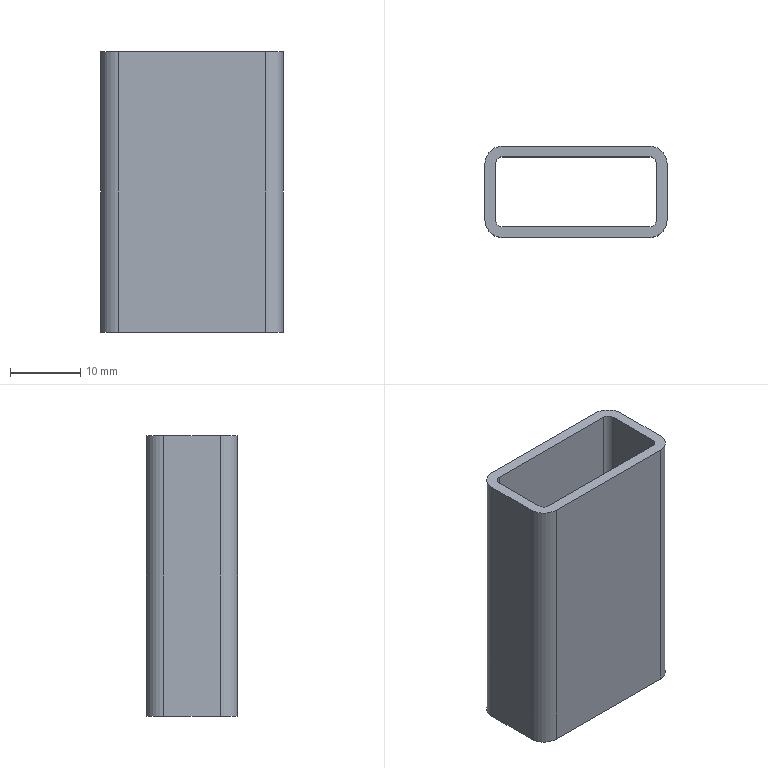Part | STEP file | 5090502 | 1 solid | 18 faces | box 26 x 13 x 40 mm | volume 4140 mm3 | plane 10 | cylinder 8 | commonest cylinder face diameters 2 x4 5 x4
STEP:
#1=CARTESIAN_POINT('',(0.,0.,0.));
#2=DIRECTION('',(0.,0.,1.));
#3=DIRECTION('',(1.,0.,0.));
#4=AXIS2_PLACEMENT_3D('',#1,#2,#3);
#5=CARTESIAN_POINT('',(13.,4.,20.));
#6=VERTEX_POINT('',#5);
#7=CARTESIAN_POINT('',(10.5,6.5,20.));
#8=VERTEX_POINT('',#7);
#9=CARTESIAN_POINT('',(10.5,4.,20.));
#10=DIRECTION('',(0.,0.,1.));
#11=DIRECTION('',(-1.,0.,0.));
#12=AXIS2_PLACEMENT_3D('',#9,#10,#11);
#13=CIRCLE('',#12,2.5);
#14=CARTESIAN_POINT('',(10.5,4.,20.));
#15=DIRECTION('',(0.,0.,-1.));
#16=DIRECTION('',(-1.,0.,0.));
#17=AXIS2_PLACEMENT_3D('',#14,#15,#16);
#18=PLANE('',#17);
#19=CARTESIAN_POINT('',(2.5,0.));
#20=CARTESIAN_POINT('',(2.5,-4.33));
#21=CARTESIAN_POINT('',(-1.25,-2.165));
#22=CARTESIAN_POINT('',(-5.,0.));
#23=CARTESIAN_POINT('',(-1.25,2.165));
#24=CARTESIAN_POINT('',(2.5,4.33));
#25=CARTESIAN_POINT('',(2.5,0.));
#26=(BOUNDED_CURVE()B_SPLINE_CURVE(2,(#19,#20,#21,#22,#23,#24,#25),.UNSPECIFIED.,.T.,.F.)B_SPLINE_CURVE_WITH_KNOTS((1,2,2,2,2,1),(-2.094,0.,2.094,4.189,6.283,8.378),.UNSPECIFIED.)CURVE()GEOMETRIC_REPRESENTATION_ITEM()RATIONAL_B_SPLINE_CURVE((1.,0.5,1.,0.5,1.,0.5,1.))REPRESENTATION_ITEM(''));
#27=(GEOMETRIC_REPRESENTATION_CONTEXT(2)PARAMETRIC_REPRESENTATION_CONTEXT()REPRESENTATION_CONTEXT('',''));
#28=DEFINITIONAL_REPRESENTATION('',(#26),#27);
#29=PCURVE('',#18,#28);
#30=CARTESIAN_POINT('',(10.5,4.,20.));
#31=DIRECTION('',(0.,0.,-1.));
#32=DIRECTION('',(-1.,0.,0.));
#33=AXIS2_PLACEMENT_3D('',#30,#31,#32);
#34=CYLINDRICAL_SURFACE('',#33,2.5);
#35=CARTESIAN_POINT('',(6.283,0.));
#36=DIRECTION('',(-1.,0.));
#37=VECTOR('',#36,1.);
#38=LINE('',#35,#37);
#39=(GEOMETRIC_REPRESENTATION_CONTEXT(2)PARAMETRIC_REPRESENTATION_CONTEXT()REPRESENTATION_CONTEXT('',''));
#40=DEFINITIONAL_REPRESENTATION('',(#38),#39);
#41=PCURVE('',#34,#40);
#42=SURFACE_CURVE('',#13,(#29,#41),.PCURVE_S1.);
#43=EDGE_CURVE('',#6,#8,#42,.T.);
#44=ORIENTED_EDGE('',*,*,#43,.T.);
#45=CARTESIAN_POINT('',(-10.5,6.5,20.));
#46=VERTEX_POINT('',#45);
#47=CARTESIAN_POINT('',(-10.5,6.5,20.));
#48=DIRECTION('',(-1.,0.,0.));
#49=VECTOR('',#48,1.);
#50=LINE('',#47,#49);
#51=CARTESIAN_POINT('',(21.,2.5));
#52=DIRECTION('',(1.,0.));
#53=VECTOR('',#52,1.);
#54=LINE('',#51,#53);
#55=(GEOMETRIC_REPRESENTATION_CONTEXT(2)PARAMETRIC_REPRESENTATION_CONTEXT()REPRESENTATION_CONTEXT('',''));
#56=DEFINITIONAL_REPRESENTATION('',(#54),#55);
#57=PCURVE('',#18,#56);
#58=CARTESIAN_POINT('',(-10.5,6.5,20.));
#59=DIRECTION('',(0.,-1.,0.));
#60=DIRECTION('',(0.,0.,-1.));
#61=AXIS2_PLACEMENT_3D('',#58,#59,#60);
#62=PLANE('',#61);
#63=CARTESIAN_POINT('',(0.,0.));
#64=DIRECTION('',(0.,-1.));
#65=VECTOR('',#64,1.);
#66=LINE('',#63,#65);
#67=(GEOMETRIC_REPRESENTATION_CONTEXT(2)PARAMETRIC_REPRESENTATION_CONTEXT()REPRESENTATION_CONTEXT('',''));
#68=DEFINITIONAL_REPRESENTATION('',(#66),#67);
#69=PCURVE('',#62,#68);
#70=SURFACE_CURVE('',#50,(#57,#69),.PCURVE_S1.);
#71=EDGE_CURVE('',#8,#46,#70,.T.);
#72=ORIENTED_EDGE('',*,*,#71,.T.);
#73=CARTESIAN_POINT('',(-13.,4.,20.));
#74=VERTEX_POINT('',#73);
#75=CARTESIAN_POINT('',(-10.5,4.,20.));
#76=DIRECTION('',(0.,0.,1.));
#77=DIRECTION('',(1.,0.,0.));
#78=AXIS2_PLACEMENT_3D('',#75,#76,#77);
#79=CIRCLE('',#78,2.5);
#80=CARTESIAN_POINT('',(18.5,0.));
#81=CARTESIAN_POINT('',(18.5,4.33));
#82=CARTESIAN_POINT('',(22.25,2.165));
#83=CARTESIAN_POINT('',(26.,0.));
#84=CARTESIAN_POINT('',(22.25,-2.165));
#85=CARTESIAN_POINT('',(18.5,-4.33));
#86=CARTESIAN_POINT('',(18.5,0.));
#87=(BOUNDED_CURVE()B_SPLINE_CURVE(2,(#80,#81,#82,#83,#84,#85,#86),.UNSPECIFIED.,.T.,.F.)B_SPLINE_CURVE_WITH_KNOTS((1,2,2,2,2,1),(-2.094,0.,2.094,4.189,6.283,8.378),.UNSPECIFIED.)CURVE()GEOMETRIC_REPRESENTATION_ITEM()RATIONAL_B_SPLINE_CURVE((1.,0.5,1.,0.5,1.,0.5,1.))REPRESENTATION_ITEM(''));
#88=(GEOMETRIC_REPRESENTATION_CONTEXT(2)PARAMETRIC_REPRESENTATION_CONTEXT()REPRESENTATION_CONTEXT('',''));
#89=DEFINITIONAL_REPRESENTATION('',(#87),#88);
#90=PCURVE('',#18,#89);
#91=CARTESIAN_POINT('',(-10.5,4.,20.));
#92=DIRECTION('',(0.,0.,-1.));
#93=DIRECTION('',(-1.,0.,0.));
#94=AXIS2_PLACEMENT_3D('',#91,#92,#93);
#95=CYLINDRICAL_SURFACE('',#94,2.5);
#96=CARTESIAN_POINT('',(3.142,0.));
#97=DIRECTION('',(-1.,0.));
#98=VECTOR('',#97,1.);
#99=LINE('',#96,#98);
#100=(GEOMETRIC_REPRESENTATION_CONTEXT(2)PARAMETRIC_REPRESENTATION_CONTEXT()REPRESENTATION_CONTEXT('',''));
#101=DEFINITIONAL_REPRESENTATION('',(#99),#100);
#102=PCURVE('',#95,#101);
#103=SURFACE_CURVE('',#79,(#90,#102),.PCURVE_S1.);
#104=EDGE_CURVE('',#46,#74,#103,.T.);
#105=ORIENTED_EDGE('',*,*,#104,.T.);
#106=CARTESIAN_POINT('',(-13.,-4.,20.));
#107=VERTEX_POINT('',#106);
#108=CARTESIAN_POINT('',(-13.,4.,20.));
#109=DIRECTION('',(0.,-1.,0.));
#110=VECTOR('',#109,1.);
#111=LINE('',#108,#110);
#112=CARTESIAN_POINT('',(23.5,0.));
#113=DIRECTION('',(0.,-1.));
#114=VECTOR('',#113,1.);
#115=LINE('',#112,#114);
#116=(GEOMETRIC_REPRESENTATION_CONTEXT(2)PARAMETRIC_REPRESENTATION_CONTEXT()REPRESENTATION_CONTEXT('',''));
#117=DEFINITIONAL_REPRESENTATION('',(#115),#116);
#118=PCURVE('',#18,#117);
#119=CARTESIAN_POINT('',(-13.,4.,20.));
#120=DIRECTION('',(1.,0.,0.));
#121=DIRECTION('',(0.,0.,-1.));
#122=AXIS2_PLACEMENT_3D('',#119,#120,#121);
#123=PLANE('',#122);
#124=CARTESIAN_POINT('',(0.,0.));
#125=DIRECTION('',(0.,-1.));
#126=VECTOR('',#125,1.);
#127=LINE('',#124,#126);
#128=(GEOMETRIC_REPRESENTATION_CONTEXT(2)PARAMETRIC_REPRESENTATION_CONTEXT()REPRESENTATION_CONTEXT('',''));
#129=DEFINITIONAL_REPRESENTATION('',(#127),#128);
#130=PCURVE('',#123,#129);
#131=SURFACE_CURVE('',#111,(#118,#130),.PCURVE_S1.);
#132=EDGE_CURVE('',#74,#107,#131,.T.);
#133=ORIENTED_EDGE('',*,*,#132,.T.);
#134=CARTESIAN_POINT('',(-10.5,-6.5,20.));
#135=VERTEX_POINT('',#134);
#136=CARTESIAN_POINT('',(-10.5,-4.,20.));
#137=DIRECTION('',(0.,0.,1.));
#138=DIRECTION('',(1.,0.,0.));
#139=AXIS2_PLACEMENT_3D('',#136,#137,#138);
#140=CIRCLE('',#139,2.5);
#141=CARTESIAN_POINT('',(18.5,-8.));
#142=CARTESIAN_POINT('',(18.5,-3.67));
#143=CARTESIAN_POINT('',(22.25,-5.835));
#144=CARTESIAN_POINT('',(26.,-8.));
#145=CARTESIAN_POINT('',(22.25,-10.165));
#146=CARTESIAN_POINT('',(18.5,-12.33));
#147=CARTESIAN_POINT('',(18.5,-8.));
#148=(BOUNDED_CURVE()B_SPLINE_CURVE(2,(#141,#142,#143,#144,#145,#146,#147),.UNSPECIFIED.,.T.,.F.)B_SPLINE_CURVE_WITH_KNOTS((1,2,2,2,2,1),(-2.094,0.,2.094,4.189,6.283,8.378),.UNSPECIFIED.)CURVE()GEOMETRIC_REPRESENTATION_ITEM()RATIONAL_B_SPLINE_CURVE((1.,0.5,1.,0.5,1.,0.5,1.))REPRESENTATION_ITEM(''));
#149=(GEOMETRIC_REPRESENTATION_CONTEXT(2)PARAMETRIC_REPRESENTATION_CONTEXT()REPRESENTATION_CONTEXT('',''));
#150=DEFINITIONAL_REPRESENTATION('',(#148),#149);
#151=PCURVE('',#18,#150);
#152=CARTESIAN_POINT('',(-10.5,-4.,20.));
#153=DIRECTION('',(0.,0.,-1.));
#154=DIRECTION('',(-1.,0.,0.));
#155=AXIS2_PLACEMENT_3D('',#152,#153,#154);
#156=CYLINDRICAL_SURFACE('',#155,2.5);
#157=CARTESIAN_POINT('',(9.425,0.));
#158=DIRECTION('',(-1.,0.));
#159=VECTOR('',#158,1.);
#160=LINE('',#157,#159);
#161=(GEOMETRIC_REPRESENTATION_CONTEXT(2)PARAMETRIC_REPRESENTATION_CONTEXT()REPRESENTATION_CONTEXT('',''));
#162=DEFINITIONAL_REPRESENTATION('',(#160),#161);
#163=PCURVE('',#156,#162);
#164=SURFACE_CURVE('',#140,(#151,#163),.PCURVE_S1.);
#165=EDGE_CURVE('',#107,#135,#164,.T.);
#166=ORIENTED_EDGE('',*,*,#165,.T.);
#167=CARTESIAN_POINT('',(10.5,-6.5,20.));
#168=VERTEX_POINT('',#167);
#169=CARTESIAN_POINT('',(-10.5,-6.5,20.));
#170=DIRECTION('',(1.,0.,0.));
#171=VECTOR('',#170,1.);
#172=LINE('',#169,#171);
#173=CARTESIAN_POINT('',(21.,-10.5));
#174=DIRECTION('',(-1.,0.));
#175=VECTOR('',#174,1.);
#176=LINE('',#173,#175);
#177=(GEOMETRIC_REPRESENTATION_CONTEXT(2)PARAMETRIC_REPRESENTATION_CONTEXT()REPRESENTATION_CONTEXT('',''));
#178=DEFINITIONAL_REPRESENTATION('',(#176),#177);
#179=PCURVE('',#18,#178);
#180=CARTESIAN_POINT('',(-10.5,-6.5,20.));
#181=DIRECTION('',(0.,1.,0.));
#182=DIRECTION('',(-1.,0.,0.));
#183=AXIS2_PLACEMENT_3D('',#180,#181,#182);
#184=PLANE('',#183);
#185=CARTESIAN_POINT('',(0.,0.));
#186=DIRECTION('',(-1.,0.));
#187=VECTOR('',#186,1.);
#188=LINE('',#185,#187);
#189=(GEOMETRIC_REPRESENTATION_CONTEXT(2)PARAMETRIC_REPRESENTATION_CONTEXT()REPRESENTATION_CONTEXT('',''));
#190=DEFINITIONAL_REPRESENTATION('',(#188),#189);
#191=PCURVE('',#184,#190);
#192=SURFACE_CURVE('',#172,(#179,#191),.PCURVE_S1.);
#193=EDGE_CURVE('',#135,#168,#192,.T.);
#194=ORIENTED_EDGE('',*,*,#193,.T.);
#195=CARTESIAN_POINT('',(13.,-4.,20.));
#196=VERTEX_POINT('',#195);
#197=CARTESIAN_POINT('',(10.5,-4.,20.));
#198=DIRECTION('',(0.,0.,1.));
#199=DIRECTION('',(-1.,0.,0.));
#200=AXIS2_PLACEMENT_3D('',#197,#198,#199);
#201=CIRCLE('',#200,2.5);
#202=CARTESIAN_POINT('',(2.5,-8.));
#203=CARTESIAN_POINT('',(2.5,-12.33));
#204=CARTESIAN_POINT('',(-1.25,-10.165));
#205=CARTESIAN_POINT('',(-5.,-8.));
#206=CARTESIAN_POINT('',(-1.25,-5.835));
#207=CARTESIAN_POINT('',(2.5,-3.67));
#208=CARTESIAN_POINT('',(2.5,-8.));
#209=(BOUNDED_CURVE()B_SPLINE_CURVE(2,(#202,#203,#204,#205,#206,#207,#208),.UNSPECIFIED.,.T.,.F.)B_SPLINE_CURVE_WITH_KNOTS((1,2,2,2,2,1),(-2.094,0.,2.094,4.189,6.283,8.378),.UNSPECIFIED.)CURVE()GEOMETRIC_REPRESENTATION_ITEM()RATIONAL_B_SPLINE_CURVE((1.,0.5,1.,0.5,1.,0.5,1.))REPRESENTATION_ITEM(''));
#210=(GEOMETRIC_REPRESENTATION_CONTEXT(2)PARAMETRIC_REPRESENTATION_CONTEXT()REPRESENTATION_CONTEXT('',''));
#211=DEFINITIONAL_REPRESENTATION('',(#209),#210);
#212=PCURVE('',#18,#211);
#213=CARTESIAN_POINT('',(10.5,-4.,20.));
#214=DIRECTION('',(0.,0.,-1.));
#215=DIRECTION('',(-1.,0.,0.));
#216=AXIS2_PLACEMENT_3D('',#213,#214,#215);
#217=CYLINDRICAL_SURFACE('',#216,2.5);
#218=CARTESIAN_POINT('',(6.283,0.));
#219=DIRECTION('',(-1.,0.));
#220=VECTOR('',#219,1.);
#221=LINE('',#218,#220);
#222=(GEOMETRIC_REPRESENTATION_CONTEXT(2)PARAMETRIC_REPRESENTATION_CONTEXT()REPRESENTATION_CONTEXT('',''));
#223=DEFINITIONAL_REPRESENTATION('',(#221),#222);
#224=PCURVE('',#217,#223);
#225=SURFACE_CURVE('',#201,(#212,#224),.PCURVE_S1.);
#226=EDGE_CURVE('',#168,#196,#225,.T.);
#227=ORIENTED_EDGE('',*,*,#226,.T.);
#228=CARTESIAN_POINT('',(13.,4.,20.));
#229=DIRECTION('',(0.,1.,0.));
#230=VECTOR('',#229,1.);
#231=LINE('',#228,#230);
#232=CARTESIAN_POINT('',(-2.5,0.));
#233=DIRECTION('',(0.,1.));
#234=VECTOR('',#233,1.);
#235=LINE('',#232,#234);
#236=(GEOMETRIC_REPRESENTATION_CONTEXT(2)PARAMETRIC_REPRESENTATION_CONTEXT()REPRESENTATION_CONTEXT('',''));
#237=DEFINITIONAL_REPRESENTATION('',(#235),#236);
#238=PCURVE('',#18,#237);
#239=CARTESIAN_POINT('',(13.,4.,20.));
#240=DIRECTION('',(-1.,0.,0.));
#241=DIRECTION('',(0.,-1.,0.));
#242=AXIS2_PLACEMENT_3D('',#239,#240,#241);
#243=PLANE('',#242);
#244=CARTESIAN_POINT('',(0.,0.));
#245=DIRECTION('',(-1.,0.));
#246=VECTOR('',#245,1.);
#247=LINE('',#244,#246);
#248=(GEOMETRIC_REPRESENTATION_CONTEXT(2)PARAMETRIC_REPRESENTATION_CONTEXT()REPRESENTATION_CONTEXT('',''));
#249=DEFINITIONAL_REPRESENTATION('',(#247),#248);
#250=PCURVE('',#243,#249);
#251=SURFACE_CURVE('',#231,(#238,#250),.PCURVE_S1.);
#252=EDGE_CURVE('',#196,#6,#251,.T.);
#253=ORIENTED_EDGE('',*,*,#252,.T.);
#254=EDGE_LOOP('',(#44,#72,#105,#133,#166,#194,#227,#253));
#255=FACE_BOUND('',#254,.T.);
#256=CARTESIAN_POINT('',(-10.5,5.,20.));
#257=VERTEX_POINT('',#256);
#258=CARTESIAN_POINT('',(-11.5,4.,20.));
#259=VERTEX_POINT('',#258);
#260=CARTESIAN_POINT('',(-10.5,4.,20.));
#261=DIRECTION('',(0.,0.,1.));
#262=DIRECTION('',(1.,0.,0.));
#263=AXIS2_PLACEMENT_3D('',#260,#261,#262);
#264=CIRCLE('',#263,1.);
#265=CARTESIAN_POINT('',(20.,0.));
#266=CARTESIAN_POINT('',(20.,1.732));
#267=CARTESIAN_POINT('',(21.5,0.866));
#268=CARTESIAN_POINT('',(23.,0.));
#269=CARTESIAN_POINT('',(21.5,-0.866));
#270=CARTESIAN_POINT('',(20.,-1.732));
#271=CARTESIAN_POINT('',(20.,0.));
#272=(BOUNDED_CURVE()B_SPLINE_CURVE(2,(#265,#266,#267,#268,#269,#270,#271),.UNSPECIFIED.,.T.,.F.)B_SPLINE_CURVE_WITH_KNOTS((1,2,2,2,2,1),(-2.094,0.,2.094,4.189,6.283,8.378),.UNSPECIFIED.)CURVE()GEOMETRIC_REPRESENTATION_ITEM()RATIONAL_B_SPLINE_CURVE((1.,0.5,1.,0.5,1.,0.5,1.))REPRESENTATION_ITEM(''));
#273=(GEOMETRIC_REPRESENTATION_CONTEXT(2)PARAMETRIC_REPRESENTATION_CONTEXT()REPRESENTATION_CONTEXT('',''));
#274=DEFINITIONAL_REPRESENTATION('',(#272),#273);
#275=PCURVE('',#18,#274);
#276=CARTESIAN_POINT('',(-10.5,4.,20.));
#277=DIRECTION('',(0.,0.,-1.));
#278=DIRECTION('',(-1.,0.,0.));
#279=AXIS2_PLACEMENT_3D('',#276,#277,#278);
#280=CYLINDRICAL_SURFACE('',#279,1.);
#281=CARTESIAN_POINT('',(3.142,0.));
#282=DIRECTION('',(-1.,0.));
#283=VECTOR('',#282,1.);
#284=LINE('',#281,#283);
#285=(GEOMETRIC_REPRESENTATION_CONTEXT(2)PARAMETRIC_REPRESENTATION_CONTEXT()REPRESENTATION_CONTEXT('',''));
#286=DEFINITIONAL_REPRESENTATION('',(#284),#285);
#287=PCURVE('',#280,#286);
#288=SURFACE_CURVE('',#264,(#275,#287),.PCURVE_S1.);
#289=EDGE_CURVE('',#257,#259,#288,.T.);
#290=ORIENTED_EDGE('',*,*,#289,.F.);
#291=CARTESIAN_POINT('',(10.5,5.,20.));
#292=VERTEX_POINT('',#291);
#293=CARTESIAN_POINT('',(-10.5,5.,20.));
#294=DIRECTION('',(-1.,0.,0.));
#295=VECTOR('',#294,1.);
#296=LINE('',#293,#295);
#297=CARTESIAN_POINT('',(21.,1.));
#298=DIRECTION('',(1.,0.));
#299=VECTOR('',#298,1.);
#300=LINE('',#297,#299);
#301=(GEOMETRIC_REPRESENTATION_CONTEXT(2)PARAMETRIC_REPRESENTATION_CONTEXT()REPRESENTATION_CONTEXT('',''));
#302=DEFINITIONAL_REPRESENTATION('',(#300),#301);
#303=PCURVE('',#18,#302);
#304=CARTESIAN_POINT('',(-10.5,5.,20.));
#305=DIRECTION('',(0.,-1.,0.));
#306=DIRECTION('',(0.,0.,-1.));
#307=AXIS2_PLACEMENT_3D('',#304,#305,#306);
#308=PLANE('',#307);
#309=CARTESIAN_POINT('',(0.,0.));
#310=DIRECTION('',(0.,-1.));
#311=VECTOR('',#310,1.);
#312=LINE('',#309,#311);
#313=(GEOMETRIC_REPRESENTATION_CONTEXT(2)PARAMETRIC_REPRESENTATION_CONTEXT()REPRESENTATION_CONTEXT('',''));
#314=DEFINITIONAL_REPRESENTATION('',(#312),#313);
#315=PCURVE('',#308,#314);
#316=SURFACE_CURVE('',#296,(#303,#315),.PCURVE_S1.);
#317=EDGE_CURVE('',#292,#257,#316,.T.);
#318=ORIENTED_EDGE('',*,*,#317,.F.);
#319=CARTESIAN_POINT('',(11.5,4.,20.));
#320=VERTEX_POINT('',#319);
#321=CARTESIAN_POINT('',(10.5,4.,20.));
#322=DIRECTION('',(0.,0.,1.));
#323=DIRECTION('',(-1.,0.,0.));
#324=AXIS2_PLACEMENT_3D('',#321,#322,#323);
#325=CIRCLE('',#324,1.);
#326=CARTESIAN_POINT('',(1.,0.));
#327=CARTESIAN_POINT('',(1.,-1.732));
#328=CARTESIAN_POINT('',(-0.5,-0.866));
#329=CARTESIAN_POINT('',(-2.,0.));
#330=CARTESIAN_POINT('',(-0.5,0.866));
#331=CARTESIAN_POINT('',(1.,1.732));
#332=CARTESIAN_POINT('',(1.,0.));
#333=(BOUNDED_CURVE()B_SPLINE_CURVE(2,(#326,#327,#328,#329,#330,#331,#332),.UNSPECIFIED.,.T.,.F.)B_SPLINE_CURVE_WITH_KNOTS((1,2,2,2,2,1),(-2.094,0.,2.094,4.189,6.283,8.378),.UNSPECIFIED.)CURVE()GEOMETRIC_REPRESENTATION_ITEM()RATIONAL_B_SPLINE_CURVE((1.,0.5,1.,0.5,1.,0.5,1.))REPRESENTATION_ITEM(''));
#334=(GEOMETRIC_REPRESENTATION_CONTEXT(2)PARAMETRIC_REPRESENTATION_CONTEXT()REPRESENTATION_CONTEXT('',''));
#335=DEFINITIONAL_REPRESENTATION('',(#333),#334);
#336=PCURVE('',#18,#335);
#337=CARTESIAN_POINT('',(10.5,4.,20.));
#338=DIRECTION('',(0.,0.,-1.));
#339=DIRECTION('',(-1.,0.,0.));
#340=AXIS2_PLACEMENT_3D('',#337,#338,#339);
#341=CYLINDRICAL_SURFACE('',#340,1.);
#342=CARTESIAN_POINT('',(6.283,0.));
#343=DIRECTION('',(-1.,0.));
#344=VECTOR('',#343,1.);
#345=LINE('',#342,#344);
#346=(GEOMETRIC_REPRESENTATION_CONTEXT(2)PARAMETRIC_REPRESENTATION_CONTEXT()REPRESENTATION_CONTEXT('',''));
#347=DEFINITIONAL_REPRESENTATION('',(#345),#346);
#348=PCURVE('',#341,#347);
#349=SURFACE_CURVE('',#325,(#336,#348),.PCURVE_S1.);
#350=EDGE_CURVE('',#320,#292,#349,.T.);
#351=ORIENTED_EDGE('',*,*,#350,.F.);
#352=CARTESIAN_POINT('',(11.5,-4.,20.));
#353=VERTEX_POINT('',#352);
#354=CARTESIAN_POINT('',(11.5,4.,20.));
#355=DIRECTION('',(0.,1.,0.));
#356=VECTOR('',#355,1.);
#357=LINE('',#354,#356);
#358=CARTESIAN_POINT('',(-1.,0.));
#359=DIRECTION('',(0.,1.));
#360=VECTOR('',#359,1.);
#361=LINE('',#358,#360);
#362=(GEOMETRIC_REPRESENTATION_CONTEXT(2)PARAMETRIC_REPRESENTATION_CONTEXT()REPRESENTATION_CONTEXT('',''));
#363=DEFINITIONAL_REPRESENTATION('',(#361),#362);
#364=PCURVE('',#18,#363);
#365=CARTESIAN_POINT('',(11.5,4.,20.));
#366=DIRECTION('',(-1.,0.,0.));
#367=DIRECTION('',(0.,-1.,0.));
#368=AXIS2_PLACEMENT_3D('',#365,#366,#367);
#369=PLANE('',#368);
#370=CARTESIAN_POINT('',(0.,0.));
#371=DIRECTION('',(-1.,0.));
#372=VECTOR('',#371,1.);
#373=LINE('',#370,#372);
#374=(GEOMETRIC_REPRESENTATION_CONTEXT(2)PARAMETRIC_REPRESENTATION_CONTEXT()REPRESENTATION_CONTEXT('',''));
#375=DEFINITIONAL_REPRESENTATION('',(#373),#374);
#376=PCURVE('',#369,#375);
#377=SURFACE_CURVE('',#357,(#364,#376),.PCURVE_S1.);
#378=EDGE_CURVE('',#353,#320,#377,.T.);
#379=ORIENTED_EDGE('',*,*,#378,.F.);
#380=CARTESIAN_POINT('',(10.5,-5.,20.));
#381=VERTEX_POINT('',#380);
#382=CARTESIAN_POINT('',(10.5,-4.,20.));
#383=DIRECTION('',(0.,0.,1.));
#384=DIRECTION('',(-1.,0.,0.));
#385=AXIS2_PLACEMENT_3D('',#382,#383,#384);
#386=CIRCLE('',#385,1.);
#387=CARTESIAN_POINT('',(1.,-8.));
#388=CARTESIAN_POINT('',(1.,-9.732));
#389=CARTESIAN_POINT('',(-0.5,-8.866));
#390=CARTESIAN_POINT('',(-2.,-8.));
#391=CARTESIAN_POINT('',(-0.5,-7.134));
#392=CARTESIAN_POINT('',(1.,-6.268));
#393=CARTESIAN_POINT('',(1.,-8.));
#394=(BOUNDED_CURVE()B_SPLINE_CURVE(2,(#387,#388,#389,#390,#391,#392,#393),.UNSPECIFIED.,.T.,.F.)B_SPLINE_CURVE_WITH_KNOTS((1,2,2,2,2,1),(-2.094,0.,2.094,4.189,6.283,8.378),.UNSPECIFIED.)CURVE()GEOMETRIC_REPRESENTATION_ITEM()RATIONAL_B_SPLINE_CURVE((1.,0.5,1.,0.5,1.,0.5,1.))REPRESENTATION_ITEM(''));
#395=(GEOMETRIC_REPRESENTATION_CONTEXT(2)PARAMETRIC_REPRESENTATION_CONTEXT()REPRESENTATION_CONTEXT('',''));
#396=DEFINITIONAL_REPRESENTATION('',(#394),#395);
#397=PCURVE('',#18,#396);
#398=CARTESIAN_POINT('',(10.5,-4.,20.));
#399=DIRECTION('',(0.,0.,-1.));
#400=DIRECTION('',(-1.,0.,0.));
#401=AXIS2_PLACEMENT_3D('',#398,#399,#400);
#402=CYLINDRICAL_SURFACE('',#401,1.);
#403=CARTESIAN_POINT('',(6.283,0.));
#404=DIRECTION('',(-1.,0.));
#405=VECTOR('',#404,1.);
#406=LINE('',#403,#405);
#407=(GEOMETRIC_REPRESENTATION_CONTEXT(2)PARAMETRIC_REPRESENTATION_CONTEXT()REPRESENTATION_CONTEXT('',''));
#408=DEFINITIONAL_REPRESENTATION('',(#406),#407);
#409=PCURVE('',#402,#408);
#410=SURFACE_CURVE('',#386,(#397,#409),.PCURVE_S1.);
#411=EDGE_CURVE('',#381,#353,#410,.T.);
#412=ORIENTED_EDGE('',*,*,#411,.F.);
#413=CARTESIAN_POINT('',(-10.5,-5.,20.));
#414=VERTEX_POINT('',#413);
#415=CARTESIAN_POINT('',(-10.5,-5.,20.));
#416=DIRECTION('',(1.,0.,0.));
#417=VECTOR('',#416,1.);
#418=LINE('',#415,#417);
#419=CARTESIAN_POINT('',(21.,-9.));
#420=DIRECTION('',(-1.,0.));
#421=VECTOR('',#420,1.);
#422=LINE('',#419,#421);
#423=(GEOMETRIC_REPRESENTATION_CONTEXT(2)PARAMETRIC_REPRESENTATION_CONTEXT()REPRESENTATION_CONTEXT('',''));
#424=DEFINITIONAL_REPRESENTATION('',(#422),#423);
#425=PCURVE('',#18,#424);
#426=CARTESIAN_POINT('',(-10.5,-5.,20.));
#427=DIRECTION('',(0.,1.,0.));
#428=DIRECTION('',(-1.,0.,0.));
#429=AXIS2_PLACEMENT_3D('',#426,#427,#428);
#430=PLANE('',#429);
#431=CARTESIAN_POINT('',(0.,0.));
#432=DIRECTION('',(-1.,0.));
#433=VECTOR('',#432,1.);
#434=LINE('',#431,#433);
#435=(GEOMETRIC_REPRESENTATION_CONTEXT(2)PARAMETRIC_REPRESENTATION_CONTEXT()REPRESENTATION_CONTEXT('',''));
#436=DEFINITIONAL_REPRESENTATION('',(#434),#435);
#437=PCURVE('',#430,#436);
#438=SURFACE_CURVE('',#418,(#425,#437),.PCURVE_S1.);
#439=EDGE_CURVE('',#414,#381,#438,.T.);
#440=ORIENTED_EDGE('',*,*,#439,.F.);
#441=CARTESIAN_POINT('',(-11.5,-4.,20.));
#442=VERTEX_POINT('',#441);
#443=CARTESIAN_POINT('',(-10.5,-4.,20.));
#444=DIRECTION('',(0.,0.,1.));
#445=DIRECTION('',(1.,0.,0.));
#446=AXIS2_PLACEMENT_3D('',#443,#444,#445);
#447=CIRCLE('',#446,1.);
#448=CARTESIAN_POINT('',(20.,-8.));
#449=CARTESIAN_POINT('',(20.,-6.268));
#450=CARTESIAN_POINT('',(21.5,-7.134));
#451=CARTESIAN_POINT('',(23.,-8.));
#452=CARTESIAN_POINT('',(21.5,-8.866));
#453=CARTESIAN_POINT('',(20.,-9.732));
#454=CARTESIAN_POINT('',(20.,-8.));
#455=(BOUNDED_CURVE()B_SPLINE_CURVE(2,(#448,#449,#450,#451,#452,#453,#454),.UNSPECIFIED.,.T.,.F.)B_SPLINE_CURVE_WITH_KNOTS((1,2,2,2,2,1),(-2.094,0.,2.094,4.189,6.283,8.378),.UNSPECIFIED.)CURVE()GEOMETRIC_REPRESENTATION_ITEM()RATIONAL_B_SPLINE_CURVE((1.,0.5,1.,0.5,1.,0.5,1.))REPRESENTATION_ITEM(''));
#456=(GEOMETRIC_REPRESENTATION_CONTEXT(2)PARAMETRIC_REPRESENTATION_CONTEXT()REPRESENTATION_CONTEXT('',''));
#457=DEFINITIONAL_REPRESENTATION('',(#455),#456);
#458=PCURVE('',#18,#457);
#459=CARTESIAN_POINT('',(-10.5,-4.,20.));
#460=DIRECTION('',(0.,0.,-1.));
#461=DIRECTION('',(-1.,0.,0.));
#462=AXIS2_PLACEMENT_3D('',#459,#460,#461);
#463=CYLINDRICAL_SURFACE('',#462,1.);
#464=CARTESIAN_POINT('',(9.425,0.));
#465=DIRECTION('',(-1.,0.));
#466=VECTOR('',#465,1.);
#467=LINE('',#464,#466);
#468=(GEOMETRIC_REPRESENTATION_CONTEXT(2)PARAMETRIC_REPRESENTATION_CONTEXT()REPRESENTATION_CONTEXT('',''));
#469=DEFINITIONAL_REPRESENTATION('',(#467),#468);
#470=PCURVE('',#463,#469);
#471=SURFACE_CURVE('',#447,(#458,#470),.PCURVE_S1.);
#472=EDGE_CURVE('',#442,#414,#471,.T.);
#473=ORIENTED_EDGE('',*,*,#472,.F.);
#474=CARTESIAN_POINT('',(-11.5,4.,20.));
#475=DIRECTION('',(0.,-1.,0.));
#476=VECTOR('',#475,1.);
#477=LINE('',#474,#476);
#478=CARTESIAN_POINT('',(22.,0.));
#479=DIRECTION('',(0.,-1.));
#480=VECTOR('',#479,1.);
#481=LINE('',#478,#480);
#482=(GEOMETRIC_REPRESENTATION_CONTEXT(2)PARAMETRIC_REPRESENTATION_CONTEXT()REPRESENTATION_CONTEXT('',''));
#483=DEFINITIONAL_REPRESENTATION('',(#481),#482);
#484=PCURVE('',#18,#483);
#485=CARTESIAN_POINT('',(-11.5,4.,20.));
#486=DIRECTION('',(1.,0.,0.));
#487=DIRECTION('',(0.,1.,0.));
#488=AXIS2_PLACEMENT_3D('',#485,#486,#487);
#489=PLANE('',#488);
#490=CARTESIAN_POINT('',(0.,0.));
#491=DIRECTION('',(-1.,0.));
#492=VECTOR('',#491,1.);
#493=LINE('',#490,#492);
#494=(GEOMETRIC_REPRESENTATION_CONTEXT(2)PARAMETRIC_REPRESENTATION_CONTEXT()REPRESENTATION_CONTEXT('',''));
#495=DEFINITIONAL_REPRESENTATION('',(#493),#494);
#496=PCURVE('',#489,#495);
#497=SURFACE_CURVE('',#477,(#484,#496),.PCURVE_S1.);
#498=EDGE_CURVE('',#259,#442,#497,.T.);
#499=ORIENTED_EDGE('',*,*,#498,.F.);
#500=EDGE_LOOP('',(#290,#318,#351,#379,#412,#440,#473,#499));
#501=FACE_BOUND('',#500,.T.);
#502=ADVANCED_FACE('',(#255,#501),#18,.F.);
#503=CARTESIAN_POINT('',(13.,4.,-20.));
#504=VERTEX_POINT('',#503);
#505=CARTESIAN_POINT('',(10.5,6.5,-20.));
#506=VERTEX_POINT('',#505);
#507=CARTESIAN_POINT('',(10.5,4.,-20.));
#508=DIRECTION('',(0.,0.,1.));
#509=DIRECTION('',(-1.,0.,0.));
#510=AXIS2_PLACEMENT_3D('',#507,#508,#509);
#511=CIRCLE('',#510,2.5);
#512=CARTESIAN_POINT('',(10.5,4.,-20.));
#513=DIRECTION('',(0.,0.,-1.));
#514=DIRECTION('',(-1.,0.,0.));
#515=AXIS2_PLACEMENT_3D('',#512,#513,#514);
#516=PLANE('',#515);
#517=CARTESIAN_POINT('',(2.5,0.));
#518=CARTESIAN_POINT('',(2.5,-4.33));
#519=CARTESIAN_POINT('',(-1.25,-2.165));
#520=CARTESIAN_POINT('',(-5.,0.));
#521=CARTESIAN_POINT('',(-1.25,2.165));
#522=CARTESIAN_POINT('',(2.5,4.33));
#523=CARTESIAN_POINT('',(2.5,0.));
#524=(BOUNDED_CURVE()B_SPLINE_CURVE(2,(#517,#518,#519,#520,#521,#522,#523),.UNSPECIFIED.,.T.,.F.)B_SPLINE_CURVE_WITH_KNOTS((1,2,2,2,2,1),(-2.094,0.,2.094,4.189,6.283,8.378),.UNSPECIFIED.)CURVE()GEOMETRIC_REPRESENTATION_ITEM()RATIONAL_B_SPLINE_CURVE((1.,0.5,1.,0.5,1.,0.5,1.))REPRESENTATION_ITEM(''));
#525=(GEOMETRIC_REPRESENTATION_CONTEXT(2)PARAMETRIC_REPRESENTATION_CONTEXT()REPRESENTATION_CONTEXT('',''));
#526=DEFINITIONAL_REPRESENTATION('',(#524),#525);
#527=PCURVE('',#516,#526);
#528=CARTESIAN_POINT('',(6.283,40.));
#529=DIRECTION('',(-1.,0.));
#530=VECTOR('',#529,1.);
#531=LINE('',#528,#530);
#532=(GEOMETRIC_REPRESENTATION_CONTEXT(2)PARAMETRIC_REPRESENTATION_CONTEXT()REPRESENTATION_CONTEXT('',''));
#533=DEFINITIONAL_REPRESENTATION('',(#531),#532);
#534=PCURVE('',#34,#533);
#535=SURFACE_CURVE('',#511,(#527,#534),.PCURVE_S1.);
#536=EDGE_CURVE('',#504,#506,#535,.T.);
#537=ORIENTED_EDGE('',*,*,#536,.F.);
#538=CARTESIAN_POINT('',(13.,-4.,-20.));
#539=VERTEX_POINT('',#538);
#540=CARTESIAN_POINT('',(13.,4.,-20.));
#541=DIRECTION('',(0.,1.,0.));
#542=VECTOR('',#541,1.);
#543=LINE('',#540,#542);
#544=CARTESIAN_POINT('',(-2.5,0.));
#545=DIRECTION('',(0.,1.));
#546=VECTOR('',#545,1.);
#547=LINE('',#544,#546);
#548=(GEOMETRIC_REPRESENTATION_CONTEXT(2)PARAMETRIC_REPRESENTATION_CONTEXT()REPRESENTATION_CONTEXT('',''));
#549=DEFINITIONAL_REPRESENTATION('',(#547),#548);
#550=PCURVE('',#516,#549);
#551=CARTESIAN_POINT('',(0.,-40.));
#552=DIRECTION('',(-1.,0.));
#553=VECTOR('',#552,1.);
#554=LINE('',#551,#553);
#555=(GEOMETRIC_REPRESENTATION_CONTEXT(2)PARAMETRIC_REPRESENTATION_CONTEXT()REPRESENTATION_CONTEXT('',''));
#556=DEFINITIONAL_REPRESENTATION('',(#554),#555);
#557=PCURVE('',#243,#556);
#558=SURFACE_CURVE('',#543,(#550,#557),.PCURVE_S1.);
#559=EDGE_CURVE('',#539,#504,#558,.T.);
#560=ORIENTED_EDGE('',*,*,#559,.F.);
#561=CARTESIAN_POINT('',(10.5,-6.5,-20.));
#562=VERTEX_POINT('',#561);
#563=CARTESIAN_POINT('',(10.5,-4.,-20.));
#564=DIRECTION('',(0.,0.,1.));
#565=DIRECTION('',(-1.,0.,0.));
#566=AXIS2_PLACEMENT_3D('',#563,#564,#565);
#567=CIRCLE('',#566,2.5);
#568=CARTESIAN_POINT('',(2.5,-8.));
#569=CARTESIAN_POINT('',(2.5,-12.33));
#570=CARTESIAN_POINT('',(-1.25,-10.165));
#571=CARTESIAN_POINT('',(-5.,-8.));
#572=CARTESIAN_POINT('',(-1.25,-5.835));
#573=CARTESIAN_POINT('',(2.5,-3.67));
#574=CARTESIAN_POINT('',(2.5,-8.));
#575=(BOUNDED_CURVE()B_SPLINE_CURVE(2,(#568,#569,#570,#571,#572,#573,#574),.UNSPECIFIED.,.T.,.F.)B_SPLINE_CURVE_WITH_KNOTS((1,2,2,2,2,1),(-2.094,0.,2.094,4.189,6.283,8.378),.UNSPECIFIED.)CURVE()GEOMETRIC_REPRESENTATION_ITEM()RATIONAL_B_SPLINE_CURVE((1.,0.5,1.,0.5,1.,0.5,1.))REPRESENTATION_ITEM(''));
#576=(GEOMETRIC_REPRESENTATION_CONTEXT(2)PARAMETRIC_REPRESENTATION_CONTEXT()REPRESENTATION_CONTEXT('',''));
#577=DEFINITIONAL_REPRESENTATION('',(#575),#576);
#578=PCURVE('',#516,#577);
#579=CARTESIAN_POINT('',(6.283,40.));
#580=DIRECTION('',(-1.,0.));
#581=VECTOR('',#580,1.);
#582=LINE('',#579,#581);
#583=(GEOMETRIC_REPRESENTATION_CONTEXT(2)PARAMETRIC_REPRESENTATION_CONTEXT()REPRESENTATION_CONTEXT('',''));
#584=DEFINITIONAL_REPRESENTATION('',(#582),#583);
#585=PCURVE('',#217,#584);
#586=SURFACE_CURVE('',#567,(#578,#585),.PCURVE_S1.);
#587=EDGE_CURVE('',#562,#539,#586,.T.);
#588=ORIENTED_EDGE('',*,*,#587,.F.);
#589=CARTESIAN_POINT('',(-10.5,-6.5,-20.));
#590=VERTEX_POINT('',#589);
#591=CARTESIAN_POINT('',(-10.5,-6.5,-20.));
#592=DIRECTION('',(1.,0.,0.));
#593=VECTOR('',#592,1.);
#594=LINE('',#591,#593);
#595=CARTESIAN_POINT('',(21.,-10.5));
#596=DIRECTION('',(-1.,0.));
#597=VECTOR('',#596,1.);
#598=LINE('',#595,#597);
#599=(GEOMETRIC_REPRESENTATION_CONTEXT(2)PARAMETRIC_REPRESENTATION_CONTEXT()REPRESENTATION_CONTEXT('',''));
#600=DEFINITIONAL_REPRESENTATION('',(#598),#599);
#601=PCURVE('',#516,#600);
#602=CARTESIAN_POINT('',(0.,-40.));
#603=DIRECTION('',(-1.,0.));
#604=VECTOR('',#603,1.);
#605=LINE('',#602,#604);
#606=(GEOMETRIC_REPRESENTATION_CONTEXT(2)PARAMETRIC_REPRESENTATION_CONTEXT()REPRESENTATION_CONTEXT('',''));
#607=DEFINITIONAL_REPRESENTATION('',(#605),#606);
#608=PCURVE('',#184,#607);
#609=SURFACE_CURVE('',#594,(#601,#608),.PCURVE_S1.);
#610=EDGE_CURVE('',#590,#562,#609,.T.);
#611=ORIENTED_EDGE('',*,*,#610,.F.);
#612=CARTESIAN_POINT('',(-13.,-4.,-20.));
#613=VERTEX_POINT('',#612);
#614=CARTESIAN_POINT('',(-10.5,-4.,-20.));
#615=DIRECTION('',(0.,0.,1.));
#616=DIRECTION('',(1.,0.,0.));
#617=AXIS2_PLACEMENT_3D('',#614,#615,#616);
#618=CIRCLE('',#617,2.5);
#619=CARTESIAN_POINT('',(18.5,-8.));
#620=CARTESIAN_POINT('',(18.5,-3.67));
#621=CARTESIAN_POINT('',(22.25,-5.835));
#622=CARTESIAN_POINT('',(26.,-8.));
#623=CARTESIAN_POINT('',(22.25,-10.165));
#624=CARTESIAN_POINT('',(18.5,-12.33));
#625=CARTESIAN_POINT('',(18.5,-8.));
#626=(BOUNDED_CURVE()B_SPLINE_CURVE(2,(#619,#620,#621,#622,#623,#624,#625),.UNSPECIFIED.,.T.,.F.)B_SPLINE_CURVE_WITH_KNOTS((1,2,2,2,2,1),(-2.094,0.,2.094,4.189,6.283,8.378),.UNSPECIFIED.)CURVE()GEOMETRIC_REPRESENTATION_ITEM()RATIONAL_B_SPLINE_CURVE((1.,0.5,1.,0.5,1.,0.5,1.))REPRESENTATION_ITEM(''));
#627=(GEOMETRIC_REPRESENTATION_CONTEXT(2)PARAMETRIC_REPRESENTATION_CONTEXT()REPRESENTATION_CONTEXT('',''));
#628=DEFINITIONAL_REPRESENTATION('',(#626),#627);
#629=PCURVE('',#516,#628);
#630=CARTESIAN_POINT('',(9.425,40.));
#631=DIRECTION('',(-1.,0.));
#632=VECTOR('',#631,1.);
#633=LINE('',#630,#632);
#634=(GEOMETRIC_REPRESENTATION_CONTEXT(2)PARAMETRIC_REPRESENTATION_CONTEXT()REPRESENTATION_CONTEXT('',''));
#635=DEFINITIONAL_REPRESENTATION('',(#633),#634);
#636=PCURVE('',#156,#635);
#637=SURFACE_CURVE('',#618,(#629,#636),.PCURVE_S1.);
#638=EDGE_CURVE('',#613,#590,#637,.T.);
#639=ORIENTED_EDGE('',*,*,#638,.F.);
#640=CARTESIAN_POINT('',(-13.,4.,-20.));
#641=VERTEX_POINT('',#640);
#642=CARTESIAN_POINT('',(-13.,4.,-20.));
#643=DIRECTION('',(0.,-1.,0.));
#644=VECTOR('',#643,1.);
#645=LINE('',#642,#644);
#646=CARTESIAN_POINT('',(23.5,0.));
#647=DIRECTION('',(0.,-1.));
#648=VECTOR('',#647,1.);
#649=LINE('',#646,#648);
#650=(GEOMETRIC_REPRESENTATION_CONTEXT(2)PARAMETRIC_REPRESENTATION_CONTEXT()REPRESENTATION_CONTEXT('',''));
#651=DEFINITIONAL_REPRESENTATION('',(#649),#650);
#652=PCURVE('',#516,#651);
#653=CARTESIAN_POINT('',(40.,0.));
#654=DIRECTION('',(0.,-1.));
#655=VECTOR('',#654,1.);
#656=LINE('',#653,#655);
#657=(GEOMETRIC_REPRESENTATION_CONTEXT(2)PARAMETRIC_REPRESENTATION_CONTEXT()REPRESENTATION_CONTEXT('',''));
#658=DEFINITIONAL_REPRESENTATION('',(#656),#657);
#659=PCURVE('',#123,#658);
#660=SURFACE_CURVE('',#645,(#652,#659),.PCURVE_S1.);
#661=EDGE_CURVE('',#641,#613,#660,.T.);
#662=ORIENTED_EDGE('',*,*,#661,.F.);
#663=CARTESIAN_POINT('',(-10.5,6.5,-20.));
#664=VERTEX_POINT('',#663);
#665=CARTESIAN_POINT('',(-10.5,4.,-20.));
#666=DIRECTION('',(0.,0.,1.));
#667=DIRECTION('',(1.,0.,0.));
#668=AXIS2_PLACEMENT_3D('',#665,#666,#667);
#669=CIRCLE('',#668,2.5);
#670=CARTESIAN_POINT('',(18.5,0.));
#671=CARTESIAN_POINT('',(18.5,4.33));
#672=CARTESIAN_POINT('',(22.25,2.165));
#673=CARTESIAN_POINT('',(26.,0.));
#674=CARTESIAN_POINT('',(22.25,-2.165));
#675=CARTESIAN_POINT('',(18.5,-4.33));
#676=CARTESIAN_POINT('',(18.5,0.));
#677=(BOUNDED_CURVE()B_SPLINE_CURVE(2,(#670,#671,#672,#673,#674,#675,#676),.UNSPECIFIED.,.T.,.F.)B_SPLINE_CURVE_WITH_KNOTS((1,2,2,2,2,1),(-2.094,0.,2.094,4.189,6.283,8.378),.UNSPECIFIED.)CURVE()GEOMETRIC_REPRESENTATION_ITEM()RATIONAL_B_SPLINE_CURVE((1.,0.5,1.,0.5,1.,0.5,1.))REPRESENTATION_ITEM(''));
#678=(GEOMETRIC_REPRESENTATION_CONTEXT(2)PARAMETRIC_REPRESENTATION_CONTEXT()REPRESENTATION_CONTEXT('',''));
#679=DEFINITIONAL_REPRESENTATION('',(#677),#678);
#680=PCURVE('',#516,#679);
#681=CARTESIAN_POINT('',(3.142,40.));
#682=DIRECTION('',(-1.,0.));
#683=VECTOR('',#682,1.);
#684=LINE('',#681,#683);
#685=(GEOMETRIC_REPRESENTATION_CONTEXT(2)PARAMETRIC_REPRESENTATION_CONTEXT()REPRESENTATION_CONTEXT('',''));
#686=DEFINITIONAL_REPRESENTATION('',(#684),#685);
#687=PCURVE('',#95,#686);
#688=SURFACE_CURVE('',#669,(#680,#687),.PCURVE_S1.);
#689=EDGE_CURVE('',#664,#641,#688,.T.);
#690=ORIENTED_EDGE('',*,*,#689,.F.);
#691=CARTESIAN_POINT('',(-10.5,6.5,-20.));
#692=DIRECTION('',(-1.,0.,0.));
#693=VECTOR('',#692,1.);
#694=LINE('',#691,#693);
#695=CARTESIAN_POINT('',(21.,2.5));
#696=DIRECTION('',(1.,0.));
#697=VECTOR('',#696,1.);
#698=LINE('',#695,#697);
#699=(GEOMETRIC_REPRESENTATION_CONTEXT(2)PARAMETRIC_REPRESENTATION_CONTEXT()REPRESENTATION_CONTEXT('',''));
#700=DEFINITIONAL_REPRESENTATION('',(#698),#699);
#701=PCURVE('',#516,#700);
#702=CARTESIAN_POINT('',(40.,0.));
#703=DIRECTION('',(0.,-1.));
#704=VECTOR('',#703,1.);
#705=LINE('',#702,#704);
#706=(GEOMETRIC_REPRESENTATION_CONTEXT(2)PARAMETRIC_REPRESENTATION_CONTEXT()REPRESENTATION_CONTEXT('',''));
#707=DEFINITIONAL_REPRESENTATION('',(#705),#706);
#708=PCURVE('',#62,#707);
#709=SURFACE_CURVE('',#694,(#701,#708),.PCURVE_S1.);
#710=EDGE_CURVE('',#506,#664,#709,.T.);
#711=ORIENTED_EDGE('',*,*,#710,.F.);
#712=EDGE_LOOP('',(#537,#560,#588,#611,#639,#662,#690,#711));
#713=FACE_BOUND('',#712,.T.);
#714=CARTESIAN_POINT('',(10.5,5.,-20.));
#715=VERTEX_POINT('',#714);
#716=CARTESIAN_POINT('',(-10.5,5.,-20.));
#717=VERTEX_POINT('',#716);
#718=CARTESIAN_POINT('',(-10.5,5.,-20.));
#719=DIRECTION('',(-1.,0.,0.));
#720=VECTOR('',#719,1.);
#721=LINE('',#718,#720);
#722=CARTESIAN_POINT('',(21.,1.));
#723=DIRECTION('',(1.,0.));
#724=VECTOR('',#723,1.);
#725=LINE('',#722,#724);
#726=(GEOMETRIC_REPRESENTATION_CONTEXT(2)PARAMETRIC_REPRESENTATION_CONTEXT()REPRESENTATION_CONTEXT('',''));
#727=DEFINITIONAL_REPRESENTATION('',(#725),#726);
#728=PCURVE('',#516,#727);
#729=CARTESIAN_POINT('',(40.,0.));
#730=DIRECTION('',(0.,-1.));
#731=VECTOR('',#730,1.);
#732=LINE('',#729,#731);
#733=(GEOMETRIC_REPRESENTATION_CONTEXT(2)PARAMETRIC_REPRESENTATION_CONTEXT()REPRESENTATION_CONTEXT('',''));
#734=DEFINITIONAL_REPRESENTATION('',(#732),#733);
#735=PCURVE('',#308,#734);
#736=SURFACE_CURVE('',#721,(#728,#735),.PCURVE_S1.);
#737=EDGE_CURVE('',#715,#717,#736,.T.);
#738=ORIENTED_EDGE('',*,*,#737,.T.);
#739=CARTESIAN_POINT('',(-11.5,4.,-20.));
#740=VERTEX_POINT('',#739);
#741=CARTESIAN_POINT('',(-10.5,4.,-20.));
#742=DIRECTION('',(0.,0.,1.));
#743=DIRECTION('',(1.,0.,0.));
#744=AXIS2_PLACEMENT_3D('',#741,#742,#743);
#745=CIRCLE('',#744,1.);
#746=CARTESIAN_POINT('',(20.,0.));
#747=CARTESIAN_POINT('',(20.,1.732));
#748=CARTESIAN_POINT('',(21.5,0.866));
#749=CARTESIAN_POINT('',(23.,0.));
#750=CARTESIAN_POINT('',(21.5,-0.866));
#751=CARTESIAN_POINT('',(20.,-1.732));
#752=CARTESIAN_POINT('',(20.,0.));
#753=(BOUNDED_CURVE()B_SPLINE_CURVE(2,(#746,#747,#748,#749,#750,#751,#752),.UNSPECIFIED.,.T.,.F.)B_SPLINE_CURVE_WITH_KNOTS((1,2,2,2,2,1),(-2.094,0.,2.094,4.189,6.283,8.378),.UNSPECIFIED.)CURVE()GEOMETRIC_REPRESENTATION_ITEM()RATIONAL_B_SPLINE_CURVE((1.,0.5,1.,0.5,1.,0.5,1.))REPRESENTATION_ITEM(''));
#754=(GEOMETRIC_REPRESENTATION_CONTEXT(2)PARAMETRIC_REPRESENTATION_CONTEXT()REPRESENTATION_CONTEXT('',''));
#755=DEFINITIONAL_REPRESENTATION('',(#753),#754);
#756=PCURVE('',#516,#755);
#757=CARTESIAN_POINT('',(3.142,40.));
#758=DIRECTION('',(-1.,0.));
#759=VECTOR('',#758,1.);
#760=LINE('',#757,#759);
#761=(GEOMETRIC_REPRESENTATION_CONTEXT(2)PARAMETRIC_REPRESENTATION_CONTEXT()REPRESENTATION_CONTEXT('',''));
#762=DEFINITIONAL_REPRESENTATION('',(#760),#761);
#763=PCURVE('',#280,#762);
#764=SURFACE_CURVE('',#745,(#756,#763),.PCURVE_S1.);
#765=EDGE_CURVE('',#717,#740,#764,.T.);
#766=ORIENTED_EDGE('',*,*,#765,.T.);
#767=CARTESIAN_POINT('',(-11.5,-4.,-20.));
#768=VERTEX_POINT('',#767);
#769=CARTESIAN_POINT('',(-11.5,4.,-20.));
#770=DIRECTION('',(0.,-1.,0.));
#771=VECTOR('',#770,1.);
#772=LINE('',#769,#771);
#773=CARTESIAN_POINT('',(22.,0.));
#774=DIRECTION('',(0.,-1.));
#775=VECTOR('',#774,1.);
#776=LINE('',#773,#775);
#777=(GEOMETRIC_REPRESENTATION_CONTEXT(2)PARAMETRIC_REPRESENTATION_CONTEXT()REPRESENTATION_CONTEXT('',''));
#778=DEFINITIONAL_REPRESENTATION('',(#776),#777);
#779=PCURVE('',#516,#778);
#780=CARTESIAN_POINT('',(0.,-40.));
#781=DIRECTION('',(-1.,0.));
#782=VECTOR('',#781,1.);
#783=LINE('',#780,#782);
#784=(GEOMETRIC_REPRESENTATION_CONTEXT(2)PARAMETRIC_REPRESENTATION_CONTEXT()REPRESENTATION_CONTEXT('',''));
#785=DEFINITIONAL_REPRESENTATION('',(#783),#784);
#786=PCURVE('',#489,#785);
#787=SURFACE_CURVE('',#772,(#779,#786),.PCURVE_S1.);
#788=EDGE_CURVE('',#740,#768,#787,.T.);
#789=ORIENTED_EDGE('',*,*,#788,.T.);
#790=CARTESIAN_POINT('',(-10.5,-5.,-20.));
#791=VERTEX_POINT('',#790);
#792=CARTESIAN_POINT('',(-10.5,-4.,-20.));
#793=DIRECTION('',(0.,0.,1.));
#794=DIRECTION('',(1.,0.,0.));
#795=AXIS2_PLACEMENT_3D('',#792,#793,#794);
#796=CIRCLE('',#795,1.);
#797=CARTESIAN_POINT('',(20.,-8.));
#798=CARTESIAN_POINT('',(20.,-6.268));
#799=CARTESIAN_POINT('',(21.5,-7.134));
#800=CARTESIAN_POINT('',(23.,-8.));
#801=CARTESIAN_POINT('',(21.5,-8.866));
#802=CARTESIAN_POINT('',(20.,-9.732));
#803=CARTESIAN_POINT('',(20.,-8.));
#804=(BOUNDED_CURVE()B_SPLINE_CURVE(2,(#797,#798,#799,#800,#801,#802,#803),.UNSPECIFIED.,.T.,.F.)B_SPLINE_CURVE_WITH_KNOTS((1,2,2,2,2,1),(-2.094,0.,2.094,4.189,6.283,8.378),.UNSPECIFIED.)CURVE()GEOMETRIC_REPRESENTATION_ITEM()RATIONAL_B_SPLINE_CURVE((1.,0.5,1.,0.5,1.,0.5,1.))REPRESENTATION_ITEM(''));
#805=(GEOMETRIC_REPRESENTATION_CONTEXT(2)PARAMETRIC_REPRESENTATION_CONTEXT()REPRESENTATION_CONTEXT('',''));
#806=DEFINITIONAL_REPRESENTATION('',(#804),#805);
#807=PCURVE('',#516,#806);
#808=CARTESIAN_POINT('',(9.425,40.));
#809=DIRECTION('',(-1.,0.));
#810=VECTOR('',#809,1.);
#811=LINE('',#808,#810);
#812=(GEOMETRIC_REPRESENTATION_CONTEXT(2)PARAMETRIC_REPRESENTATION_CONTEXT()REPRESENTATION_CONTEXT('',''));
#813=DEFINITIONAL_REPRESENTATION('',(#811),#812);
#814=PCURVE('',#463,#813);
#815=SURFACE_CURVE('',#796,(#807,#814),.PCURVE_S1.);
#816=EDGE_CURVE('',#768,#791,#815,.T.);
#817=ORIENTED_EDGE('',*,*,#816,.T.);
#818=CARTESIAN_POINT('',(10.5,-5.,-20.));
#819=VERTEX_POINT('',#818);
#820=CARTESIAN_POINT('',(-10.5,-5.,-20.));
#821=DIRECTION('',(1.,0.,0.));
#822=VECTOR('',#821,1.);
#823=LINE('',#820,#822);
#824=CARTESIAN_POINT('',(21.,-9.));
#825=DIRECTION('',(-1.,0.));
#826=VECTOR('',#825,1.);
#827=LINE('',#824,#826);
#828=(GEOMETRIC_REPRESENTATION_CONTEXT(2)PARAMETRIC_REPRESENTATION_CONTEXT()REPRESENTATION_CONTEXT('',''));
#829=DEFINITIONAL_REPRESENTATION('',(#827),#828);
#830=PCURVE('',#516,#829);
#831=CARTESIAN_POINT('',(0.,-40.));
#832=DIRECTION('',(-1.,0.));
#833=VECTOR('',#832,1.);
#834=LINE('',#831,#833);
#835=(GEOMETRIC_REPRESENTATION_CONTEXT(2)PARAMETRIC_REPRESENTATION_CONTEXT()REPRESENTATION_CONTEXT('',''));
#836=DEFINITIONAL_REPRESENTATION('',(#834),#835);
#837=PCURVE('',#430,#836);
#838=SURFACE_CURVE('',#823,(#830,#837),.PCURVE_S1.);
#839=EDGE_CURVE('',#791,#819,#838,.T.);
#840=ORIENTED_EDGE('',*,*,#839,.T.);
#841=CARTESIAN_POINT('',(11.5,-4.,-20.));
#842=VERTEX_POINT('',#841);
#843=CARTESIAN_POINT('',(10.5,-4.,-20.));
#844=DIRECTION('',(0.,0.,1.));
#845=DIRECTION('',(-1.,0.,0.));
#846=AXIS2_PLACEMENT_3D('',#843,#844,#845);
#847=CIRCLE('',#846,1.);
#848=CARTESIAN_POINT('',(1.,-8.));
#849=CARTESIAN_POINT('',(1.,-9.732));
#850=CARTESIAN_POINT('',(-0.5,-8.866));
#851=CARTESIAN_POINT('',(-2.,-8.));
#852=CARTESIAN_POINT('',(-0.5,-7.134));
#853=CARTESIAN_POINT('',(1.,-6.268));
#854=CARTESIAN_POINT('',(1.,-8.));
#855=(BOUNDED_CURVE()B_SPLINE_CURVE(2,(#848,#849,#850,#851,#852,#853,#854),.UNSPECIFIED.,.T.,.F.)B_SPLINE_CURVE_WITH_KNOTS((1,2,2,2,2,1),(-2.094,0.,2.094,4.189,6.283,8.378),.UNSPECIFIED.)CURVE()GEOMETRIC_REPRESENTATION_ITEM()RATIONAL_B_SPLINE_CURVE((1.,0.5,1.,0.5,1.,0.5,1.))REPRESENTATION_ITEM(''));
#856=(GEOMETRIC_REPRESENTATION_CONTEXT(2)PARAMETRIC_REPRESENTATION_CONTEXT()REPRESENTATION_CONTEXT('',''));
#857=DEFINITIONAL_REPRESENTATION('',(#855),#856);
#858=PCURVE('',#516,#857);
#859=CARTESIAN_POINT('',(6.283,40.));
#860=DIRECTION('',(-1.,0.));
#861=VECTOR('',#860,1.);
#862=LINE('',#859,#861);
#863=(GEOMETRIC_REPRESENTATION_CONTEXT(2)PARAMETRIC_REPRESENTATION_CONTEXT()REPRESENTATION_CONTEXT('',''));
#864=DEFINITIONAL_REPRESENTATION('',(#862),#863);
#865=PCURVE('',#402,#864);
#866=SURFACE_CURVE('',#847,(#858,#865),.PCURVE_S1.);
#867=EDGE_CURVE('',#819,#842,#866,.T.);
#868=ORIENTED_EDGE('',*,*,#867,.T.);
#869=CARTESIAN_POINT('',(11.5,4.,-20.));
#870=VERTEX_POINT('',#869);
#871=CARTESIAN_POINT('',(11.5,4.,-20.));
#872=DIRECTION('',(0.,1.,0.));
#873=VECTOR('',#872,1.);
#874=LINE('',#871,#873);
#875=CARTESIAN_POINT('',(-1.,0.));
#876=DIRECTION('',(0.,1.));
#877=VECTOR('',#876,1.);
#878=LINE('',#875,#877);
#879=(GEOMETRIC_REPRESENTATION_CONTEXT(2)PARAMETRIC_REPRESENTATION_CONTEXT()REPRESENTATION_CONTEXT('',''));
#880=DEFINITIONAL_REPRESENTATION('',(#878),#879);
#881=PCURVE('',#516,#880);
#882=CARTESIAN_POINT('',(0.,-40.));
#883=DIRECTION('',(-1.,0.));
#884=VECTOR('',#883,1.);
#885=LINE('',#882,#884);
#886=(GEOMETRIC_REPRESENTATION_CONTEXT(2)PARAMETRIC_REPRESENTATION_CONTEXT()REPRESENTATION_CONTEXT('',''));
#887=DEFINITIONAL_REPRESENTATION('',(#885),#886);
#888=PCURVE('',#369,#887);
#889=SURFACE_CURVE('',#874,(#881,#888),.PCURVE_S1.);
#890=EDGE_CURVE('',#842,#870,#889,.T.);
#891=ORIENTED_EDGE('',*,*,#890,.T.);
#892=CARTESIAN_POINT('',(10.5,4.,-20.));
#893=DIRECTION('',(0.,0.,1.));
#894=DIRECTION('',(-1.,0.,0.));
#895=AXIS2_PLACEMENT_3D('',#892,#893,#894);
#896=CIRCLE('',#895,1.);
#897=CARTESIAN_POINT('',(1.,0.));
#898=CARTESIAN_POINT('',(1.,-1.732));
#899=CARTESIAN_POINT('',(-0.5,-0.866));
#900=CARTESIAN_POINT('',(-2.,0.));
#901=CARTESIAN_POINT('',(-0.5,0.866));
#902=CARTESIAN_POINT('',(1.,1.732));
#903=CARTESIAN_POINT('',(1.,0.));
#904=(BOUNDED_CURVE()B_SPLINE_CURVE(2,(#897,#898,#899,#900,#901,#902,#903),.UNSPECIFIED.,.T.,.F.)B_SPLINE_CURVE_WITH_KNOTS((1,2,2,2,2,1),(-2.094,0.,2.094,4.189,6.283,8.378),.UNSPECIFIED.)CURVE()GEOMETRIC_REPRESENTATION_ITEM()RATIONAL_B_SPLINE_CURVE((1.,0.5,1.,0.5,1.,0.5,1.))REPRESENTATION_ITEM(''));
#905=(GEOMETRIC_REPRESENTATION_CONTEXT(2)PARAMETRIC_REPRESENTATION_CONTEXT()REPRESENTATION_CONTEXT('',''));
#906=DEFINITIONAL_REPRESENTATION('',(#904),#905);
#907=PCURVE('',#516,#906);
#908=CARTESIAN_POINT('',(6.283,40.));
#909=DIRECTION('',(-1.,0.));
#910=VECTOR('',#909,1.);
#911=LINE('',#908,#910);
#912=(GEOMETRIC_REPRESENTATION_CONTEXT(2)PARAMETRIC_REPRESENTATION_CONTEXT()REPRESENTATION_CONTEXT('',''));
#913=DEFINITIONAL_REPRESENTATION('',(#911),#912);
#914=PCURVE('',#341,#913);
#915=SURFACE_CURVE('',#896,(#907,#914),.PCURVE_S1.);
#916=EDGE_CURVE('',#870,#715,#915,.T.);
#917=ORIENTED_EDGE('',*,*,#916,.T.);
#918=EDGE_LOOP('',(#738,#766,#789,#817,#840,#868,#891,#917));
#919=FACE_BOUND('',#918,.T.);
#920=ADVANCED_FACE('',(#713,#919),#516,.T.);
#921=ORIENTED_EDGE('',*,*,#536,.T.);
#922=CARTESIAN_POINT('',(10.5,6.5,20.));
#923=DIRECTION('',(0.,0.,-1.));
#924=VECTOR('',#923,1.);
#925=LINE('',#922,#924);
#926=CARTESIAN_POINT('',(1.571,0.));
#927=DIRECTION('',(0.,1.));
#928=VECTOR('',#927,1.);
#929=LINE('',#926,#928);
#930=(GEOMETRIC_REPRESENTATION_CONTEXT(2)PARAMETRIC_REPRESENTATION_CONTEXT()REPRESENTATION_CONTEXT('',''));
#931=DEFINITIONAL_REPRESENTATION('',(#929),#930);
#932=PCURVE('',#34,#931);
#933=CARTESIAN_POINT('',(0.,21.));
#934=DIRECTION('',(1.,0.));
#935=VECTOR('',#934,1.);
#936=LINE('',#933,#935);
#937=(GEOMETRIC_REPRESENTATION_CONTEXT(2)PARAMETRIC_REPRESENTATION_CONTEXT()REPRESENTATION_CONTEXT('',''));
#938=DEFINITIONAL_REPRESENTATION('',(#936),#937);
#939=PCURVE('',#62,#938);
#940=SURFACE_CURVE('',#925,(#932,#939),.PCURVE_S1.);
#941=EDGE_CURVE('',#8,#506,#940,.T.);
#942=ORIENTED_EDGE('',*,*,#941,.F.);
#943=ORIENTED_EDGE('',*,*,#43,.F.);
#944=CARTESIAN_POINT('',(13.,4.,20.));
#945=DIRECTION('',(0.,0.,-1.));
#946=VECTOR('',#945,1.);
#947=LINE('',#944,#946);
#948=CARTESIAN_POINT('',(3.142,0.));
#949=DIRECTION('',(0.,1.));
#950=VECTOR('',#949,1.);
#951=LINE('',#948,#950);
#952=(GEOMETRIC_REPRESENTATION_CONTEXT(2)PARAMETRIC_REPRESENTATION_CONTEXT()REPRESENTATION_CONTEXT('',''));
#953=DEFINITIONAL_REPRESENTATION('',(#951),#952);
#954=PCURVE('',#34,#953);
#955=CARTESIAN_POINT('',(0.,0.));
#956=DIRECTION('',(0.,-1.));
#957=VECTOR('',#956,1.);
#958=LINE('',#955,#957);
#959=(GEOMETRIC_REPRESENTATION_CONTEXT(2)PARAMETRIC_REPRESENTATION_CONTEXT()REPRESENTATION_CONTEXT('',''));
#960=DEFINITIONAL_REPRESENTATION('',(#958),#959);
#961=PCURVE('',#243,#960);
#962=SURFACE_CURVE('',#947,(#954,#961),.PCURVE_S1.);
#963=EDGE_CURVE('',#6,#504,#962,.T.);
#964=ORIENTED_EDGE('',*,*,#963,.T.);
#965=EDGE_LOOP('',(#921,#942,#943,#964));
#966=FACE_BOUND('',#965,.T.);
#967=ADVANCED_FACE('',(#966),#34,.T.);
#968=ORIENTED_EDGE('',*,*,#710,.T.);
#969=CARTESIAN_POINT('',(-10.5,6.5,20.));
#970=DIRECTION('',(0.,0.,-1.));
#971=VECTOR('',#970,1.);
#972=LINE('',#969,#971);
#973=CARTESIAN_POINT('',(0.,0.));
#974=DIRECTION('',(1.,0.));
#975=VECTOR('',#974,1.);
#976=LINE('',#973,#975);
#977=(GEOMETRIC_REPRESENTATION_CONTEXT(2)PARAMETRIC_REPRESENTATION_CONTEXT()REPRESENTATION_CONTEXT('',''));
#978=DEFINITIONAL_REPRESENTATION('',(#976),#977);
#979=PCURVE('',#62,#978);
#980=CARTESIAN_POINT('',(1.571,0.));
#981=DIRECTION('',(0.,1.));
#982=VECTOR('',#981,1.);
#983=LINE('',#980,#982);
#984=(GEOMETRIC_REPRESENTATION_CONTEXT(2)PARAMETRIC_REPRESENTATION_CONTEXT()REPRESENTATION_CONTEXT('',''));
#985=DEFINITIONAL_REPRESENTATION('',(#983),#984);
#986=PCURVE('',#95,#985);
#987=SURFACE_CURVE('',#972,(#979,#986),.PCURVE_S1.);
#988=EDGE_CURVE('',#46,#664,#987,.T.);
#989=ORIENTED_EDGE('',*,*,#988,.F.);
#990=ORIENTED_EDGE('',*,*,#71,.F.);
#991=ORIENTED_EDGE('',*,*,#941,.T.);
#992=EDGE_LOOP('',(#968,#989,#990,#991));
#993=FACE_BOUND('',#992,.T.);
#994=ADVANCED_FACE('',(#993),#62,.F.);
#995=ORIENTED_EDGE('',*,*,#689,.T.);
#996=CARTESIAN_POINT('',(-13.,4.,20.));
#997=DIRECTION('',(0.,0.,-1.));
#998=VECTOR('',#997,1.);
#999=LINE('',#996,#998);
#1000=CARTESIAN_POINT('',(0.,0.));
#1001=DIRECTION('',(0.,1.));
#1002=VECTOR('',#1001,1.);
#1003=LINE('',#1000,#1002);
#1004=(GEOMETRIC_REPRESENTATION_CONTEXT(2)PARAMETRIC_REPRESENTATION_CONTEXT()REPRESENTATION_CONTEXT('',''));
#1005=DEFINITIONAL_REPRESENTATION('',(#1003),#1004);
#1006=PCURVE('',#95,#1005);
#1007=CARTESIAN_POINT('',(0.,0.));
#1008=DIRECTION('',(1.,0.));
#1009=VECTOR('',#1008,1.);
#1010=LINE('',#1007,#1009);
#1011=(GEOMETRIC_REPRESENTATION_CONTEXT(2)PARAMETRIC_REPRESENTATION_CONTEXT()REPRESENTATION_CONTEXT('',''));
#1012=DEFINITIONAL_REPRESENTATION('',(#1010),#1011);
#1013=PCURVE('',#123,#1012);
#1014=SURFACE_CURVE('',#999,(#1006,#1013),.PCURVE_S1.);
#1015=EDGE_CURVE('',#74,#641,#1014,.T.);
#1016=ORIENTED_EDGE('',*,*,#1015,.F.);
#1017=ORIENTED_EDGE('',*,*,#104,.F.);
#1018=ORIENTED_EDGE('',*,*,#988,.T.);
#1019=EDGE_LOOP('',(#995,#1016,#1017,#1018));
#1020=FACE_BOUND('',#1019,.T.);
#1021=ADVANCED_FACE('',(#1020),#95,.T.);
#1022=ORIENTED_EDGE('',*,*,#661,.T.);
#1023=CARTESIAN_POINT('',(-13.,-4.,20.));
#1024=DIRECTION('',(0.,0.,-1.));
#1025=VECTOR('',#1024,1.);
#1026=LINE('',#1023,#1025);
#1027=CARTESIAN_POINT('',(0.,-8.));
#1028=DIRECTION('',(1.,0.));
#1029=VECTOR('',#1028,1.);
#1030=LINE('',#1027,#1029);
#1031=(GEOMETRIC_REPRESENTATION_CONTEXT(2)PARAMETRIC_REPRESENTATION_CONTEXT()REPRESENTATION_CONTEXT('',''));
#1032=DEFINITIONAL_REPRESENTATION('',(#1030),#1031);
#1033=PCURVE('',#123,#1032);
#1034=CARTESIAN_POINT('',(6.283,0.));
#1035=DIRECTION('',(0.,1.));
#1036=VECTOR('',#1035,1.);
#1037=LINE('',#1034,#1036);
#1038=(GEOMETRIC_REPRESENTATION_CONTEXT(2)PARAMETRIC_REPRESENTATION_CONTEXT()REPRESENTATION_CONTEXT('',''));
#1039=DEFINITIONAL_REPRESENTATION('',(#1037),#1038);
#1040=PCURVE('',#156,#1039);
#1041=SURFACE_CURVE('',#1026,(#1033,#1040),.PCURVE_S1.);
#1042=EDGE_CURVE('',#107,#613,#1041,.T.);
#1043=ORIENTED_EDGE('',*,*,#1042,.F.);
#1044=ORIENTED_EDGE('',*,*,#132,.F.);
#1045=ORIENTED_EDGE('',*,*,#1015,.T.);
#1046=EDGE_LOOP('',(#1022,#1043,#1044,#1045));
#1047=FACE_BOUND('',#1046,.T.);
#1048=ADVANCED_FACE('',(#1047),#123,.F.);
#1049=ORIENTED_EDGE('',*,*,#638,.T.);
#1050=CARTESIAN_POINT('',(-10.5,-6.5,20.));
#1051=DIRECTION('',(0.,0.,-1.));
#1052=VECTOR('',#1051,1.);
#1053=LINE('',#1050,#1052);
#1054=CARTESIAN_POINT('',(4.712,0.));
#1055=DIRECTION('',(0.,1.));
#1056=VECTOR('',#1055,1.);
#1057=LINE('',#1054,#1056);
#1058=(GEOMETRIC_REPRESENTATION_CONTEXT(2)PARAMETRIC_REPRESENTATION_CONTEXT()REPRESENTATION_CONTEXT('',''));
#1059=DEFINITIONAL_REPRESENTATION('',(#1057),#1058);
#1060=PCURVE('',#156,#1059);
#1061=CARTESIAN_POINT('',(0.,0.));
#1062=DIRECTION('',(0.,-1.));
#1063=VECTOR('',#1062,1.);
#1064=LINE('',#1061,#1063);
#1065=(GEOMETRIC_REPRESENTATION_CONTEXT(2)PARAMETRIC_REPRESENTATION_CONTEXT()REPRESENTATION_CONTEXT('',''));
#1066=DEFINITIONAL_REPRESENTATION('',(#1064),#1065);
#1067=PCURVE('',#184,#1066);
#1068=SURFACE_CURVE('',#1053,(#1060,#1067),.PCURVE_S1.);
#1069=EDGE_CURVE('',#135,#590,#1068,.T.);
#1070=ORIENTED_EDGE('',*,*,#1069,.F.);
#1071=ORIENTED_EDGE('',*,*,#165,.F.);
#1072=ORIENTED_EDGE('',*,*,#1042,.T.);
#1073=EDGE_LOOP('',(#1049,#1070,#1071,#1072));
#1074=FACE_BOUND('',#1073,.T.);
#1075=ADVANCED_FACE('',(#1074),#156,.T.);
#1076=ORIENTED_EDGE('',*,*,#610,.T.);
#1077=CARTESIAN_POINT('',(10.5,-6.5,20.));
#1078=DIRECTION('',(0.,0.,-1.));
#1079=VECTOR('',#1078,1.);
#1080=LINE('',#1077,#1079);
#1081=CARTESIAN_POINT('',(-21.,0.));
#1082=DIRECTION('',(0.,-1.));
#1083=VECTOR('',#1082,1.);
#1084=LINE('',#1081,#1083);
#1085=(GEOMETRIC_REPRESENTATION_CONTEXT(2)PARAMETRIC_REPRESENTATION_CONTEXT()REPRESENTATION_CONTEXT('',''));
#1086=DEFINITIONAL_REPRESENTATION('',(#1084),#1085);
#1087=PCURVE('',#184,#1086);
#1088=CARTESIAN_POINT('',(4.712,0.));
#1089=DIRECTION('',(0.,1.));
#1090=VECTOR('',#1089,1.);
#1091=LINE('',#1088,#1090);
#1092=(GEOMETRIC_REPRESENTATION_CONTEXT(2)PARAMETRIC_REPRESENTATION_CONTEXT()REPRESENTATION_CONTEXT('',''));
#1093=DEFINITIONAL_REPRESENTATION('',(#1091),#1092);
#1094=PCURVE('',#217,#1093);
#1095=SURFACE_CURVE('',#1080,(#1087,#1094),.PCURVE_S1.);
#1096=EDGE_CURVE('',#168,#562,#1095,.T.);
#1097=ORIENTED_EDGE('',*,*,#1096,.F.);
#1098=ORIENTED_EDGE('',*,*,#193,.F.);
#1099=ORIENTED_EDGE('',*,*,#1069,.T.);
#1100=EDGE_LOOP('',(#1076,#1097,#1098,#1099));
#1101=FACE_BOUND('',#1100,.T.);
#1102=ADVANCED_FACE('',(#1101),#184,.F.);
#1103=ORIENTED_EDGE('',*,*,#587,.T.);
#1104=CARTESIAN_POINT('',(13.,-4.,20.));
#1105=DIRECTION('',(0.,0.,-1.));
#1106=VECTOR('',#1105,1.);
#1107=LINE('',#1104,#1106);
#1108=CARTESIAN_POINT('',(3.142,0.));
#1109=DIRECTION('',(0.,1.));
#1110=VECTOR('',#1109,1.);
#1111=LINE('',#1108,#1110);
#1112=(GEOMETRIC_REPRESENTATION_CONTEXT(2)PARAMETRIC_REPRESENTATION_CONTEXT()REPRESENTATION_CONTEXT('',''));
#1113=DEFINITIONAL_REPRESENTATION('',(#1111),#1112);
#1114=PCURVE('',#217,#1113);
#1115=CARTESIAN_POINT('',(8.,0.));
#1116=DIRECTION('',(0.,-1.));
#1117=VECTOR('',#1116,1.);
#1118=LINE('',#1115,#1117);
#1119=(GEOMETRIC_REPRESENTATION_CONTEXT(2)PARAMETRIC_REPRESENTATION_CONTEXT()REPRESENTATION_CONTEXT('',''));
#1120=DEFINITIONAL_REPRESENTATION('',(#1118),#1119);
#1121=PCURVE('',#243,#1120);
#1122=SURFACE_CURVE('',#1107,(#1114,#1121),.PCURVE_S1.);
#1123=EDGE_CURVE('',#196,#539,#1122,.T.);
#1124=ORIENTED_EDGE('',*,*,#1123,.F.);
#1125=ORIENTED_EDGE('',*,*,#226,.F.);
#1126=ORIENTED_EDGE('',*,*,#1096,.T.);
#1127=EDGE_LOOP('',(#1103,#1124,#1125,#1126));
#1128=FACE_BOUND('',#1127,.T.);
#1129=ADVANCED_FACE('',(#1128),#217,.T.);
#1130=ORIENTED_EDGE('',*,*,#559,.T.);
#1131=ORIENTED_EDGE('',*,*,#963,.F.);
#1132=ORIENTED_EDGE('',*,*,#252,.F.);
#1133=ORIENTED_EDGE('',*,*,#1123,.T.);
#1134=EDGE_LOOP('',(#1130,#1131,#1132,#1133));
#1135=FACE_BOUND('',#1134,.T.);
#1136=ADVANCED_FACE('',(#1135),#243,.F.);
#1137=CARTESIAN_POINT('',(-11.5,4.,20.));
#1138=DIRECTION('',(0.,0.,-1.));
#1139=VECTOR('',#1138,1.);
#1140=LINE('',#1137,#1139);
#1141=CARTESIAN_POINT('',(0.,0.));
#1142=DIRECTION('',(0.,1.));
#1143=VECTOR('',#1142,1.);
#1144=LINE('',#1141,#1143);
#1145=(GEOMETRIC_REPRESENTATION_CONTEXT(2)PARAMETRIC_REPRESENTATION_CONTEXT()REPRESENTATION_CONTEXT('',''));
#1146=DEFINITIONAL_REPRESENTATION('',(#1144),#1145);
#1147=PCURVE('',#280,#1146);
#1148=CARTESIAN_POINT('',(0.,0.));
#1149=DIRECTION('',(0.,-1.));
#1150=VECTOR('',#1149,1.);
#1151=LINE('',#1148,#1150);
#1152=(GEOMETRIC_REPRESENTATION_CONTEXT(2)PARAMETRIC_REPRESENTATION_CONTEXT()REPRESENTATION_CONTEXT('',''));
#1153=DEFINITIONAL_REPRESENTATION('',(#1151),#1152);
#1154=PCURVE('',#489,#1153);
#1155=SURFACE_CURVE('',#1140,(#1147,#1154),.PCURVE_S1.);
#1156=EDGE_CURVE('',#259,#740,#1155,.T.);
#1157=ORIENTED_EDGE('',*,*,#1156,.F.);
#1158=ORIENTED_EDGE('',*,*,#289,.F.);
#1159=CARTESIAN_POINT('',(-10.5,5.,20.));
#1160=DIRECTION('',(0.,0.,-1.));
#1161=VECTOR('',#1160,1.);
#1162=LINE('',#1159,#1161);
#1163=CARTESIAN_POINT('',(1.571,0.));
#1164=DIRECTION('',(0.,1.));
#1165=VECTOR('',#1164,1.);
#1166=LINE('',#1163,#1165);
#1167=(GEOMETRIC_REPRESENTATION_CONTEXT(2)PARAMETRIC_REPRESENTATION_CONTEXT()REPRESENTATION_CONTEXT('',''));
#1168=DEFINITIONAL_REPRESENTATION('',(#1166),#1167);
#1169=PCURVE('',#280,#1168);
#1170=CARTESIAN_POINT('',(0.,0.));
#1171=DIRECTION('',(1.,0.));
#1172=VECTOR('',#1171,1.);
#1173=LINE('',#1170,#1172);
#1174=(GEOMETRIC_REPRESENTATION_CONTEXT(2)PARAMETRIC_REPRESENTATION_CONTEXT()REPRESENTATION_CONTEXT('',''));
#1175=DEFINITIONAL_REPRESENTATION('',(#1173),#1174);
#1176=PCURVE('',#308,#1175);
#1177=SURFACE_CURVE('',#1162,(#1169,#1176),.PCURVE_S1.);
#1178=EDGE_CURVE('',#257,#717,#1177,.T.);
#1179=ORIENTED_EDGE('',*,*,#1178,.T.);
#1180=ORIENTED_EDGE('',*,*,#765,.T.);
#1181=EDGE_LOOP('',(#1157,#1158,#1179,#1180));
#1182=FACE_BOUND('',#1181,.F.);
#1183=ADVANCED_FACE('',(#1182),#280,.F.);
#1184=ORIENTED_EDGE('',*,*,#788,.F.);
#1185=ORIENTED_EDGE('',*,*,#1156,.F.);
#1186=ORIENTED_EDGE('',*,*,#498,.T.);
#1187=CARTESIAN_POINT('',(-11.5,-4.,20.));
#1188=DIRECTION('',(0.,0.,-1.));
#1189=VECTOR('',#1188,1.);
#1190=LINE('',#1187,#1189);
#1191=CARTESIAN_POINT('',(-8.,0.));
#1192=DIRECTION('',(0.,-1.));
#1193=VECTOR('',#1192,1.);
#1194=LINE('',#1191,#1193);
#1195=(GEOMETRIC_REPRESENTATION_CONTEXT(2)PARAMETRIC_REPRESENTATION_CONTEXT()REPRESENTATION_CONTEXT('',''));
#1196=DEFINITIONAL_REPRESENTATION('',(#1194),#1195);
#1197=PCURVE('',#489,#1196);
#1198=CARTESIAN_POINT('',(6.283,0.));
#1199=DIRECTION('',(0.,1.));
#1200=VECTOR('',#1199,1.);
#1201=LINE('',#1198,#1200);
#1202=(GEOMETRIC_REPRESENTATION_CONTEXT(2)PARAMETRIC_REPRESENTATION_CONTEXT()REPRESENTATION_CONTEXT('',''));
#1203=DEFINITIONAL_REPRESENTATION('',(#1201),#1202);
#1204=PCURVE('',#463,#1203);
#1205=SURFACE_CURVE('',#1190,(#1197,#1204),.PCURVE_S1.);
#1206=EDGE_CURVE('',#442,#768,#1205,.T.);
#1207=ORIENTED_EDGE('',*,*,#1206,.T.);
#1208=EDGE_LOOP('',(#1184,#1185,#1186,#1207));
#1209=FACE_BOUND('',#1208,.T.);
#1210=ADVANCED_FACE('',(#1209),#489,.T.);
#1211=CARTESIAN_POINT('',(-10.5,-5.,20.));
#1212=DIRECTION('',(0.,0.,-1.));
#1213=VECTOR('',#1212,1.);
#1214=LINE('',#1211,#1213);
#1215=CARTESIAN_POINT('',(4.712,0.));
#1216=DIRECTION('',(0.,1.));
#1217=VECTOR('',#1216,1.);
#1218=LINE('',#1215,#1217);
#1219=(GEOMETRIC_REPRESENTATION_CONTEXT(2)PARAMETRIC_REPRESENTATION_CONTEXT()REPRESENTATION_CONTEXT('',''));
#1220=DEFINITIONAL_REPRESENTATION('',(#1218),#1219);
#1221=PCURVE('',#463,#1220);
#1222=CARTESIAN_POINT('',(0.,0.));
#1223=DIRECTION('',(0.,-1.));
#1224=VECTOR('',#1223,1.);
#1225=LINE('',#1222,#1224);
#1226=(GEOMETRIC_REPRESENTATION_CONTEXT(2)PARAMETRIC_REPRESENTATION_CONTEXT()REPRESENTATION_CONTEXT('',''));
#1227=DEFINITIONAL_REPRESENTATION('',(#1225),#1226);
#1228=PCURVE('',#430,#1227);
#1229=SURFACE_CURVE('',#1214,(#1221,#1228),.PCURVE_S1.);
#1230=EDGE_CURVE('',#414,#791,#1229,.T.);
#1231=ORIENTED_EDGE('',*,*,#1230,.F.);
#1232=ORIENTED_EDGE('',*,*,#472,.F.);
#1233=ORIENTED_EDGE('',*,*,#1206,.T.);
#1234=ORIENTED_EDGE('',*,*,#816,.T.);
#1235=EDGE_LOOP('',(#1231,#1232,#1233,#1234));
#1236=FACE_BOUND('',#1235,.F.);
#1237=ADVANCED_FACE('',(#1236),#463,.F.);
#1238=ORIENTED_EDGE('',*,*,#839,.F.);
#1239=ORIENTED_EDGE('',*,*,#1230,.F.);
#1240=ORIENTED_EDGE('',*,*,#439,.T.);
#1241=CARTESIAN_POINT('',(10.5,-5.,20.));
#1242=DIRECTION('',(0.,0.,-1.));
#1243=VECTOR('',#1242,1.);
#1244=LINE('',#1241,#1243);
#1245=CARTESIAN_POINT('',(-21.,0.));
#1246=DIRECTION('',(0.,-1.));
#1247=VECTOR('',#1246,1.);
#1248=LINE('',#1245,#1247);
#1249=(GEOMETRIC_REPRESENTATION_CONTEXT(2)PARAMETRIC_REPRESENTATION_CONTEXT()REPRESENTATION_CONTEXT('',''));
#1250=DEFINITIONAL_REPRESENTATION('',(#1248),#1249);
#1251=PCURVE('',#430,#1250);
#1252=CARTESIAN_POINT('',(4.712,0.));
#1253=DIRECTION('',(0.,1.));
#1254=VECTOR('',#1253,1.);
#1255=LINE('',#1252,#1254);
#1256=(GEOMETRIC_REPRESENTATION_CONTEXT(2)PARAMETRIC_REPRESENTATION_CONTEXT()REPRESENTATION_CONTEXT('',''));
#1257=DEFINITIONAL_REPRESENTATION('',(#1255),#1256);
#1258=PCURVE('',#402,#1257);
#1259=SURFACE_CURVE('',#1244,(#1251,#1258),.PCURVE_S1.);
#1260=EDGE_CURVE('',#381,#819,#1259,.T.);
#1261=ORIENTED_EDGE('',*,*,#1260,.T.);
#1262=EDGE_LOOP('',(#1238,#1239,#1240,#1261));
#1263=FACE_BOUND('',#1262,.T.);
#1264=ADVANCED_FACE('',(#1263),#430,.T.);
#1265=CARTESIAN_POINT('',(11.5,-4.,20.));
#1266=DIRECTION('',(0.,0.,-1.));
#1267=VECTOR('',#1266,1.);
#1268=LINE('',#1265,#1267);
#1269=CARTESIAN_POINT('',(3.142,0.));
#1270=DIRECTION('',(0.,1.));
#1271=VECTOR('',#1270,1.);
#1272=LINE('',#1269,#1271);
#1273=(GEOMETRIC_REPRESENTATION_CONTEXT(2)PARAMETRIC_REPRESENTATION_CONTEXT()REPRESENTATION_CONTEXT('',''));
#1274=DEFINITIONAL_REPRESENTATION('',(#1272),#1273);
#1275=PCURVE('',#402,#1274);
#1276=CARTESIAN_POINT('',(8.,0.));
#1277=DIRECTION('',(0.,-1.));
#1278=VECTOR('',#1277,1.);
#1279=LINE('',#1276,#1278);
#1280=(GEOMETRIC_REPRESENTATION_CONTEXT(2)PARAMETRIC_REPRESENTATION_CONTEXT()REPRESENTATION_CONTEXT('',''));
#1281=DEFINITIONAL_REPRESENTATION('',(#1279),#1280);
#1282=PCURVE('',#369,#1281);
#1283=SURFACE_CURVE('',#1268,(#1275,#1282),.PCURVE_S1.);
#1284=EDGE_CURVE('',#353,#842,#1283,.T.);
#1285=ORIENTED_EDGE('',*,*,#1284,.F.);
#1286=ORIENTED_EDGE('',*,*,#411,.F.);
#1287=ORIENTED_EDGE('',*,*,#1260,.T.);
#1288=ORIENTED_EDGE('',*,*,#867,.T.);
#1289=EDGE_LOOP('',(#1285,#1286,#1287,#1288));
#1290=FACE_BOUND('',#1289,.F.);
#1291=ADVANCED_FACE('',(#1290),#402,.F.);
#1292=ORIENTED_EDGE('',*,*,#890,.F.);
#1293=ORIENTED_EDGE('',*,*,#1284,.F.);
#1294=ORIENTED_EDGE('',*,*,#378,.T.);
#1295=CARTESIAN_POINT('',(11.5,4.,20.));
#1296=DIRECTION('',(0.,0.,-1.));
#1297=VECTOR('',#1296,1.);
#1298=LINE('',#1295,#1297);
#1299=CARTESIAN_POINT('',(0.,0.));
#1300=DIRECTION('',(0.,-1.));
#1301=VECTOR('',#1300,1.);
#1302=LINE('',#1299,#1301);
#1303=(GEOMETRIC_REPRESENTATION_CONTEXT(2)PARAMETRIC_REPRESENTATION_CONTEXT()REPRESENTATION_CONTEXT('',''));
#1304=DEFINITIONAL_REPRESENTATION('',(#1302),#1303);
#1305=PCURVE('',#369,#1304);
#1306=CARTESIAN_POINT('',(3.142,0.));
#1307=DIRECTION('',(0.,1.));
#1308=VECTOR('',#1307,1.);
#1309=LINE('',#1306,#1308);
#1310=(GEOMETRIC_REPRESENTATION_CONTEXT(2)PARAMETRIC_REPRESENTATION_CONTEXT()REPRESENTATION_CONTEXT('',''));
#1311=DEFINITIONAL_REPRESENTATION('',(#1309),#1310);
#1312=PCURVE('',#341,#1311);
#1313=SURFACE_CURVE('',#1298,(#1305,#1312),.PCURVE_S1.);
#1314=EDGE_CURVE('',#320,#870,#1313,.T.);
#1315=ORIENTED_EDGE('',*,*,#1314,.T.);
#1316=EDGE_LOOP('',(#1292,#1293,#1294,#1315));
#1317=FACE_BOUND('',#1316,.T.);
#1318=ADVANCED_FACE('',(#1317),#369,.T.);
#1319=CARTESIAN_POINT('',(10.5,5.,20.));
#1320=DIRECTION('',(0.,0.,-1.));
#1321=VECTOR('',#1320,1.);
#1322=LINE('',#1319,#1321);
#1323=CARTESIAN_POINT('',(1.571,0.));
#1324=DIRECTION('',(0.,1.));
#1325=VECTOR('',#1324,1.);
#1326=LINE('',#1323,#1325);
#1327=(GEOMETRIC_REPRESENTATION_CONTEXT(2)PARAMETRIC_REPRESENTATION_CONTEXT()REPRESENTATION_CONTEXT('',''));
#1328=DEFINITIONAL_REPRESENTATION('',(#1326),#1327);
#1329=PCURVE('',#341,#1328);
#1330=CARTESIAN_POINT('',(0.,21.));
#1331=DIRECTION('',(1.,0.));
#1332=VECTOR('',#1331,1.);
#1333=LINE('',#1330,#1332);
#1334=(GEOMETRIC_REPRESENTATION_CONTEXT(2)PARAMETRIC_REPRESENTATION_CONTEXT()REPRESENTATION_CONTEXT('',''));
#1335=DEFINITIONAL_REPRESENTATION('',(#1333),#1334);
#1336=PCURVE('',#308,#1335);
#1337=SURFACE_CURVE('',#1322,(#1329,#1336),.PCURVE_S1.);
#1338=EDGE_CURVE('',#292,#715,#1337,.T.);
#1339=ORIENTED_EDGE('',*,*,#1338,.F.);
#1340=ORIENTED_EDGE('',*,*,#350,.F.);
#1341=ORIENTED_EDGE('',*,*,#1314,.T.);
#1342=ORIENTED_EDGE('',*,*,#916,.T.);
#1343=EDGE_LOOP('',(#1339,#1340,#1341,#1342));
#1344=FACE_BOUND('',#1343,.F.);
#1345=ADVANCED_FACE('',(#1344),#341,.F.);
#1346=ORIENTED_EDGE('',*,*,#737,.F.);
#1347=ORIENTED_EDGE('',*,*,#1338,.F.);
#1348=ORIENTED_EDGE('',*,*,#317,.T.);
#1349=ORIENTED_EDGE('',*,*,#1178,.T.);
#1350=EDGE_LOOP('',(#1346,#1347,#1348,#1349));
#1351=FACE_BOUND('',#1350,.T.);
#1352=ADVANCED_FACE('',(#1351),#308,.T.);
#1353=CLOSED_SHELL('',(#502,#920,#967,#994,#1021,#1048,#1075,#1102,#1129,#1136,#1183,#1210,#1237,#1264,#1291,#1318,#1345,#1352));
#1354=MANIFOLD_SOLID_BREP('',#1353);
#1355=(LENGTH_UNIT()NAMED_UNIT(*)SI_UNIT(.MILLI.,.METRE.));
#1356=UNCERTAINTY_MEASURE_WITH_UNIT(LENGTH_MEASURE(0.0000001),#1355,'','');
#1357=(NAMED_UNIT(*)PLANE_ANGLE_UNIT()SI_UNIT($,.RADIAN.));
#1358=(NAMED_UNIT(*)SI_UNIT($,.STERADIAN.)SOLID_ANGLE_UNIT());
#1359=(GEOMETRIC_REPRESENTATION_CONTEXT(3)GLOBAL_UNCERTAINTY_ASSIGNED_CONTEXT((#1356))GLOBAL_UNIT_ASSIGNED_CONTEXT((#1355,#1357,#1358))REPRESENTATION_CONTEXT('',''));
#1360=ADVANCED_BREP_SHAPE_REPRESENTATION('',(#4,#1354),#1359);